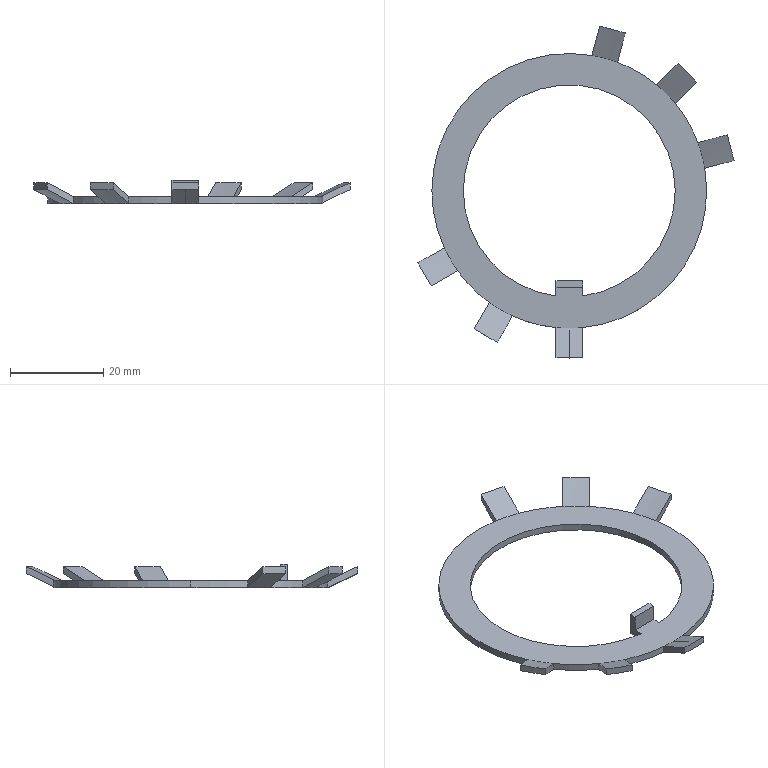Part | SolidWorks | features BaseBody 1 | 1 solid | 49 faces | box 67.906 x 71.289 x 5 mm | volume 2051 mm3 | plane 25 | cone 14 | cylinder 10 | commonest cylinder face diameters 59 x7 45.5 x3
STEP:
#1=CARTESIAN_POINT('',(0.,-29.5,0.));
#2=VERTEX_POINT('',#1);
#3=CARTESIAN_POINT('',(-2.85,-29.362,0.));
#4=VERTEX_POINT('',#3);
#5=CARTESIAN_POINT('',(0.,0.,0.));
#6=DIRECTION('',(0.,0.,-1.));
#7=DIRECTION('',(0.,1.,0.));
#8=AXIS2_PLACEMENT_3D('',#5,#6,#7);
#9=CIRCLE('',#8,29.5);
#10=EDGE_CURVE('',#2,#4,#9,.T.);
#11=ORIENTED_EDGE('',*,*,#10,.F.);
#12=CARTESIAN_POINT('',(0.,-35.887,2.978));
#13=VERTEX_POINT('',#12);
#14=CARTESIAN_POINT('',(0.,-29.5,0.));
#15=DIRECTION('',(0.,-0.9063,0.4226));
#16=VECTOR('',#15,1000.);
#17=LINE('',#14,#16);
#18=EDGE_CURVE('',#2,#13,#17,.T.);
#19=ORIENTED_EDGE('',*,*,#18,.T.);
#20=CARTESIAN_POINT('',(-2.85,-35.887,3.031));
#21=VERTEX_POINT('',#20);
#22=CARTESIAN_POINT('',(0.,-35.887,2.978));
#23=CARTESIAN_POINT('',(-0.9492,-35.887,2.978));
#24=CARTESIAN_POINT('',(-1.9,-35.887,2.996));
#25=CARTESIAN_POINT('',(-2.85,-35.887,3.031));
#26=B_SPLINE_CURVE_WITH_KNOTS('',3,(#22,#23,#24,#25),.UNSPECIFIED.,.F.,.F.,(4,4),(0.01069,0.01354),.UNSPECIFIED.);
#27=EDGE_CURVE('',#13,#21,#26,.T.);
#28=ORIENTED_EDGE('',*,*,#27,.T.);
#29=CARTESIAN_POINT('',(-2.85,-35.887,3.031));
#30=CARTESIAN_POINT('',(-2.85,-33.712,2.02));
#31=CARTESIAN_POINT('',(-2.85,-31.537,1.01));
#32=CARTESIAN_POINT('',(-2.85,-29.362,0.));
#33=B_SPLINE_CURVE_WITH_KNOTS('',3,(#29,#30,#31,#32),.UNSPECIFIED.,.F.,.F.,(4,4),(0.01329,0.02049),.UNSPECIFIED.);
#34=EDGE_CURVE('',#21,#4,#33,.T.);
#35=ORIENTED_EDGE('',*,*,#34,.T.);
#36=EDGE_LOOP('',(#11,#19,#28,#35));
#37=FACE_OUTER_BOUND('',#36,.T.);
#38=CARTESIAN_POINT('',(0.,0.,0.));
#39=DIRECTION('',(0.,0.,1.));
#40=DIRECTION('',(0.,-1.,0.));
#41=AXIS2_PLACEMENT_3D('',#38,#39,#40);
#42=CONICAL_SURFACE('',#41,29.5,1.134);
#43=ADVANCED_FACE('',(#37),#42,.T.);
#44=CARTESIAN_POINT('',(-26.853,-12.213,1.5));
#45=VERTEX_POINT('',#44);
#46=CARTESIAN_POINT('',(-29.5,0.,1.5));
#47=VERTEX_POINT('',#46);
#48=CARTESIAN_POINT('',(0.,0.,1.5));
#49=DIRECTION('',(0.,0.,-1.));
#50=DIRECTION('',(0.,1.,0.));
#51=AXIS2_PLACEMENT_3D('',#48,#49,#50);
#52=CIRCLE('',#51,29.5);
#53=EDGE_CURVE('',#45,#47,#52,.T.);
#54=ORIENTED_EDGE('',*,*,#53,.T.);
#55=CARTESIAN_POINT('',(-29.5,0.,0.));
#56=VERTEX_POINT('',#55);
#57=CARTESIAN_POINT('',(-29.5,0.,4.532));
#58=DIRECTION('',(0.,0.,-1.));
#59=VECTOR('',#58,1000.);
#60=LINE('',#57,#59);
#61=EDGE_CURVE('',#47,#56,#60,.T.);
#62=ORIENTED_EDGE('',*,*,#61,.T.);
#63=CARTESIAN_POINT('',(-26.853,-12.213,0.));
#64=VERTEX_POINT('',#63);
#65=CARTESIAN_POINT('',(0.,0.,0.));
#66=DIRECTION('',(0.,0.,1.));
#67=DIRECTION('',(1.,0.,0.));
#68=AXIS2_PLACEMENT_3D('',#65,#66,#67);
#69=CIRCLE('',#68,29.5);
#70=EDGE_CURVE('',#56,#64,#69,.T.);
#71=ORIENTED_EDGE('',*,*,#70,.T.);
#72=CARTESIAN_POINT('',(-26.853,-12.213,4.532));
#73=DIRECTION('',(0.,0.,-1.));
#74=VECTOR('',#73,1000.);
#75=LINE('',#72,#74);
#76=EDGE_CURVE('',#45,#64,#75,.T.);
#77=ORIENTED_EDGE('',*,*,#76,.F.);
#78=EDGE_LOOP('',(#54,#62,#71,#77));
#79=FACE_OUTER_BOUND('',#78,.T.);
#80=CARTESIAN_POINT('',(0.,0.,4.532));
#81=DIRECTION('',(0.,0.,-1.));
#82=DIRECTION('',(-1.,0.,0.));
#83=AXIS2_PLACEMENT_3D('',#80,#81,#82);
#84=CYLINDRICAL_SURFACE('',#83,29.5);
#85=ADVANCED_FACE('',(#79),#84,.T.);
#86=CARTESIAN_POINT('',(2.85,-22.571,1.5));
#87=VERTEX_POINT('',#86);
#88=CARTESIAN_POINT('',(22.75,0.,1.5));
#89=VERTEX_POINT('',#88);
#90=CARTESIAN_POINT('',(0.,0.,1.5));
#91=DIRECTION('',(0.,0.,1.));
#92=DIRECTION('',(0.,-1.,0.));
#93=AXIS2_PLACEMENT_3D('',#90,#91,#92);
#94=CIRCLE('',#93,22.75);
#95=EDGE_CURVE('',#87,#89,#94,.T.);
#96=ORIENTED_EDGE('',*,*,#95,.T.);
#97=CARTESIAN_POINT('',(22.75,0.,0.));
#98=VERTEX_POINT('',#97);
#99=CARTESIAN_POINT('',(22.75,0.,4.532));
#100=DIRECTION('',(0.,0.,-1.));
#101=VECTOR('',#100,1000.);
#102=LINE('',#99,#101);
#103=EDGE_CURVE('',#89,#98,#102,.T.);
#104=ORIENTED_EDGE('',*,*,#103,.T.);
#105=CARTESIAN_POINT('',(2.85,-22.571,0.));
#106=VERTEX_POINT('',#105);
#107=CARTESIAN_POINT('',(0.,0.,0.));
#108=DIRECTION('',(0.,0.,1.));
#109=DIRECTION('',(1.,0.,0.));
#110=AXIS2_PLACEMENT_3D('',#107,#108,#109);
#111=CIRCLE('',#110,22.75);
#112=EDGE_CURVE('',#106,#98,#111,.T.);
#113=ORIENTED_EDGE('',*,*,#112,.F.);
#114=CARTESIAN_POINT('',(2.85,-22.571,4.532));
#115=DIRECTION('',(0.,0.,-1.));
#116=VECTOR('',#115,1000.);
#117=LINE('',#114,#116);
#118=EDGE_CURVE('',#87,#106,#117,.T.);
#119=ORIENTED_EDGE('',*,*,#118,.F.);
#120=EDGE_LOOP('',(#96,#104,#113,#119));
#121=FACE_OUTER_BOUND('',#120,.T.);
#122=CARTESIAN_POINT('',(0.,0.,4.532));
#123=DIRECTION('',(0.,0.,-1.));
#124=DIRECTION('',(-1.,0.,0.));
#125=AXIS2_PLACEMENT_3D('',#122,#123,#124);
#126=CYLINDRICAL_SURFACE('',#125,22.75);
#127=ADVANCED_FACE('',(#121),#126,.F.);
#128=ORIENTED_EDGE('',*,*,#103,.F.);
#129=CARTESIAN_POINT('',(-22.75,0.,1.5));
#130=VERTEX_POINT('',#129);
#131=CARTESIAN_POINT('',(0.,0.,1.5));
#132=DIRECTION('',(0.,0.,1.));
#133=DIRECTION('',(0.,-1.,0.));
#134=AXIS2_PLACEMENT_3D('',#131,#132,#133);
#135=CIRCLE('',#134,22.75);
#136=EDGE_CURVE('',#89,#130,#135,.T.);
#137=ORIENTED_EDGE('',*,*,#136,.T.);
#138=CARTESIAN_POINT('',(-22.75,0.,0.));
#139=VERTEX_POINT('',#138);
#140=CARTESIAN_POINT('',(-22.75,0.,4.532));
#141=DIRECTION('',(0.,0.,-1.));
#142=VECTOR('',#141,1000.);
#143=LINE('',#140,#142);
#144=EDGE_CURVE('',#130,#139,#143,.T.);
#145=ORIENTED_EDGE('',*,*,#144,.T.);
#146=CARTESIAN_POINT('',(0.,0.,0.));
#147=DIRECTION('',(0.,0.,1.));
#148=DIRECTION('',(1.,0.,0.));
#149=AXIS2_PLACEMENT_3D('',#146,#147,#148);
#150=CIRCLE('',#149,22.75);
#151=EDGE_CURVE('',#98,#139,#150,.T.);
#152=ORIENTED_EDGE('',*,*,#151,.F.);
#153=EDGE_LOOP('',(#128,#137,#145,#152));
#154=FACE_OUTER_BOUND('',#153,.T.);
#155=CARTESIAN_POINT('',(0.,0.,4.532));
#156=DIRECTION('',(0.,0.,-1.));
#157=DIRECTION('',(-1.,0.,0.));
#158=AXIS2_PLACEMENT_3D('',#155,#156,#157);
#159=CYLINDRICAL_SURFACE('',#158,22.75);
#160=ADVANCED_FACE('',(#154),#159,.F.);
#161=CARTESIAN_POINT('',(2.85,-29.362,1.5));
#162=VERTEX_POINT('',#161);
#163=CARTESIAN_POINT('',(0.,-29.5,1.5));
#164=VERTEX_POINT('',#163);
#165=CARTESIAN_POINT('',(0.,0.,1.5));
#166=DIRECTION('',(0.,0.,-1.));
#167=DIRECTION('',(0.,1.,0.));
#168=AXIS2_PLACEMENT_3D('',#165,#166,#167);
#169=CIRCLE('',#168,29.5);
#170=EDGE_CURVE('',#162,#164,#169,.T.);
#171=ORIENTED_EDGE('',*,*,#170,.T.);
#172=CARTESIAN_POINT('',(0.,-35.887,4.478));
#173=VERTEX_POINT('',#172);
#174=CARTESIAN_POINT('',(0.,-36.,4.531));
#175=DIRECTION('',(0.,-0.9063,0.4226));
#176=VECTOR('',#175,1000.);
#177=LINE('',#174,#176);
#178=EDGE_CURVE('',#164,#173,#177,.T.);
#179=ORIENTED_EDGE('',*,*,#178,.T.);
#180=CARTESIAN_POINT('',(2.85,-35.887,4.531));
#181=VERTEX_POINT('',#180);
#182=CARTESIAN_POINT('',(0.,-35.887,4.478));
#183=CARTESIAN_POINT('',(0.951,-35.887,4.478));
#184=CARTESIAN_POINT('',(1.901,-35.887,4.496));
#185=CARTESIAN_POINT('',(2.85,-35.887,4.531));
#186=B_SPLINE_CURVE_WITH_KNOTS('',3,(#182,#183,#184,#185),.UNSPECIFIED.,.F.,.F.,(4,4),(0.01491,0.01776),.UNSPECIFIED.);
#187=EDGE_CURVE('',#173,#181,#186,.T.);
#188=ORIENTED_EDGE('',*,*,#187,.T.);
#189=CARTESIAN_POINT('',(2.85,-35.887,4.531));
#190=CARTESIAN_POINT('',(2.85,-33.712,3.52));
#191=CARTESIAN_POINT('',(2.85,-31.537,2.51));
#192=CARTESIAN_POINT('',(2.85,-29.362,1.5));
#193=B_SPLINE_CURVE_WITH_KNOTS('',3,(#189,#190,#191,#192),.UNSPECIFIED.,.F.,.F.,(4,4),(0.01329,0.02049),.UNSPECIFIED.);
#194=EDGE_CURVE('',#181,#162,#193,.T.);
#195=ORIENTED_EDGE('',*,*,#194,.T.);
#196=EDGE_LOOP('',(#171,#179,#188,#195));
#197=FACE_OUTER_BOUND('',#196,.T.);
#198=CARTESIAN_POINT('',(0.,0.,4.531));
#199=DIRECTION('',(0.,0.,1.));
#200=DIRECTION('',(0.,-1.,0.));
#201=AXIS2_PLACEMENT_3D('',#198,#199,#200);
#202=CONICAL_SURFACE('',#201,36.,1.134);
#203=ADVANCED_FACE('',(#197),#202,.F.);
#204=CARTESIAN_POINT('',(4.847,29.099,1.5));
#205=VERTEX_POINT('',#204);
#206=CARTESIAN_POINT('',(10.352,27.624,1.5));
#207=VERTEX_POINT('',#206);
#208=CARTESIAN_POINT('',(0.,0.,1.5));
#209=DIRECTION('',(0.,0.,-1.));
#210=DIRECTION('',(0.,1.,0.));
#211=AXIS2_PLACEMENT_3D('',#208,#209,#210);
#212=CIRCLE('',#211,29.5);
#213=EDGE_CURVE('',#205,#207,#212,.T.);
#214=ORIENTED_EDGE('',*,*,#213,.F.);
#215=CARTESIAN_POINT('',(0.,0.,1.5));
#216=DIRECTION('',(0.,0.,-1.));
#217=DIRECTION('',(0.,1.,0.));
#218=AXIS2_PLACEMENT_3D('',#215,#216,#217);
#219=CIRCLE('',#218,29.5);
#220=EDGE_CURVE('',#47,#205,#219,.T.);
#221=ORIENTED_EDGE('',*,*,#220,.F.);
#222=ORIENTED_EDGE('',*,*,#53,.F.);
#223=CARTESIAN_POINT('',(-24.003,-17.149,1.5));
#224=VERTEX_POINT('',#223);
#225=CARTESIAN_POINT('',(0.,0.,1.5));
#226=DIRECTION('',(0.,0.,-1.));
#227=DIRECTION('',(0.,1.,0.));
#228=AXIS2_PLACEMENT_3D('',#225,#226,#227);
#229=CIRCLE('',#228,29.5);
#230=EDGE_CURVE('',#224,#45,#229,.T.);
#231=ORIENTED_EDGE('',*,*,#230,.F.);
#232=CARTESIAN_POINT('',(-17.149,-24.003,1.5));
#233=VERTEX_POINT('',#232);
#234=CARTESIAN_POINT('',(0.,0.,1.5));
#235=DIRECTION('',(0.,0.,-1.));
#236=DIRECTION('',(0.,1.,0.));
#237=AXIS2_PLACEMENT_3D('',#234,#235,#236);
#238=CIRCLE('',#237,29.5);
#239=EDGE_CURVE('',#233,#224,#238,.T.);
#240=ORIENTED_EDGE('',*,*,#239,.F.);
#241=CARTESIAN_POINT('',(-12.213,-26.853,1.5));
#242=VERTEX_POINT('',#241);
#243=CARTESIAN_POINT('',(0.,0.,1.5));
#244=DIRECTION('',(0.,0.,-1.));
#245=DIRECTION('',(0.,1.,0.));
#246=AXIS2_PLACEMENT_3D('',#243,#244,#245);
#247=CIRCLE('',#246,29.5);
#248=EDGE_CURVE('',#242,#233,#247,.T.);
#249=ORIENTED_EDGE('',*,*,#248,.F.);
#250=CARTESIAN_POINT('',(-2.85,-29.362,1.5));
#251=VERTEX_POINT('',#250);
#252=CARTESIAN_POINT('',(0.,0.,1.5));
#253=DIRECTION('',(0.,0.,-1.));
#254=DIRECTION('',(0.,1.,0.));
#255=AXIS2_PLACEMENT_3D('',#252,#253,#254);
#256=CIRCLE('',#255,29.5);
#257=EDGE_CURVE('',#251,#242,#256,.T.);
#258=ORIENTED_EDGE('',*,*,#257,.F.);
#259=CARTESIAN_POINT('',(0.,0.,1.5));
#260=DIRECTION('',(0.,0.,-1.));
#261=DIRECTION('',(0.,1.,0.));
#262=AXIS2_PLACEMENT_3D('',#259,#260,#261);
#263=CIRCLE('',#262,29.5);
#264=EDGE_CURVE('',#164,#251,#263,.T.);
#265=ORIENTED_EDGE('',*,*,#264,.F.);
#266=ORIENTED_EDGE('',*,*,#170,.F.);
#267=CARTESIAN_POINT('',(29.099,4.847,1.5));
#268=VERTEX_POINT('',#267);
#269=CARTESIAN_POINT('',(0.,0.,1.5));
#270=DIRECTION('',(0.,0.,-1.));
#271=DIRECTION('',(0.,1.,0.));
#272=AXIS2_PLACEMENT_3D('',#269,#270,#271);
#273=CIRCLE('',#272,29.5);
#274=EDGE_CURVE('',#268,#162,#273,.T.);
#275=ORIENTED_EDGE('',*,*,#274,.F.);
#276=CARTESIAN_POINT('',(27.624,10.352,1.5));
#277=VERTEX_POINT('',#276);
#278=CARTESIAN_POINT('',(0.,0.,1.5));
#279=DIRECTION('',(0.,0.,-1.));
#280=DIRECTION('',(0.,1.,0.));
#281=AXIS2_PLACEMENT_3D('',#278,#279,#280);
#282=CIRCLE('',#281,29.5);
#283=EDGE_CURVE('',#277,#268,#282,.T.);
#284=ORIENTED_EDGE('',*,*,#283,.F.);
#285=CARTESIAN_POINT('',(22.777,18.747,1.5));
#286=VERTEX_POINT('',#285);
#287=CARTESIAN_POINT('',(0.,0.,1.5));
#288=DIRECTION('',(0.,0.,-1.));
#289=DIRECTION('',(0.,1.,0.));
#290=AXIS2_PLACEMENT_3D('',#287,#288,#289);
#291=CIRCLE('',#290,29.5);
#292=EDGE_CURVE('',#286,#277,#291,.T.);
#293=ORIENTED_EDGE('',*,*,#292,.F.);
#294=CARTESIAN_POINT('',(18.747,22.777,1.5));
#295=VERTEX_POINT('',#294);
#296=CARTESIAN_POINT('',(0.,0.,1.5));
#297=DIRECTION('',(0.,0.,-1.));
#298=DIRECTION('',(0.,1.,0.));
#299=AXIS2_PLACEMENT_3D('',#296,#297,#298);
#300=CIRCLE('',#299,29.5);
#301=EDGE_CURVE('',#295,#286,#300,.T.);
#302=ORIENTED_EDGE('',*,*,#301,.F.);
#303=CARTESIAN_POINT('',(0.,0.,1.5));
#304=DIRECTION('',(0.,0.,-1.));
#305=DIRECTION('',(0.,1.,0.));
#306=AXIS2_PLACEMENT_3D('',#303,#304,#305);
#307=CIRCLE('',#306,29.5);
#308=EDGE_CURVE('',#207,#295,#307,.T.);
#309=ORIENTED_EDGE('',*,*,#308,.F.);
#310=EDGE_LOOP('',(#214,#221,#222,#231,#240,#249,#258,#265,#266,#275,#284,#293,#302,#309));
#311=FACE_OUTER_BOUND('',#310,.T.);
#312=CARTESIAN_POINT('',(2.85,-20.75,1.5));
#313=VERTEX_POINT('',#312);
#314=CARTESIAN_POINT('',(2.85,-22.571,1.5));
#315=DIRECTION('',(0.,-1.,0.));
#316=VECTOR('',#315,1000.);
#317=LINE('',#314,#316);
#318=EDGE_CURVE('',#313,#87,#317,.T.);
#319=ORIENTED_EDGE('',*,*,#318,.F.);
#320=CARTESIAN_POINT('',(-2.85,-20.75,1.5));
#321=VERTEX_POINT('',#320);
#322=CARTESIAN_POINT('',(0.,-20.75,1.5));
#323=DIRECTION('',(-1.,0.,0.));
#324=VECTOR('',#323,1000.);
#325=LINE('',#322,#324);
#326=EDGE_CURVE('',#313,#321,#325,.T.);
#327=ORIENTED_EDGE('',*,*,#326,.T.);
#328=CARTESIAN_POINT('',(-2.85,-22.571,1.5));
#329=VERTEX_POINT('',#328);
#330=CARTESIAN_POINT('',(-2.85,-22.571,1.5));
#331=DIRECTION('',(0.,1.,0.));
#332=VECTOR('',#331,1000.);
#333=LINE('',#330,#332);
#334=EDGE_CURVE('',#329,#321,#333,.T.);
#335=ORIENTED_EDGE('',*,*,#334,.F.);
#336=CARTESIAN_POINT('',(0.,0.,1.5));
#337=DIRECTION('',(0.,0.,1.));
#338=DIRECTION('',(0.,-1.,0.));
#339=AXIS2_PLACEMENT_3D('',#336,#337,#338);
#340=CIRCLE('',#339,22.75);
#341=EDGE_CURVE('',#130,#329,#340,.T.);
#342=ORIENTED_EDGE('',*,*,#341,.F.);
#343=ORIENTED_EDGE('',*,*,#136,.F.);
#344=ORIENTED_EDGE('',*,*,#95,.F.);
#345=EDGE_LOOP('',(#319,#327,#335,#342,#343,#344));
#346=FACE_BOUND('',#345,.T.);
#347=CARTESIAN_POINT('',(0.,29.5,1.5));
#348=DIRECTION('',(0.,0.,1.));
#349=DIRECTION('',(0.,-1.,0.));
#350=AXIS2_PLACEMENT_3D('',#347,#348,#349);
#351=PLANE('',#350);
#352=ADVANCED_FACE('',(#311,#346),#351,.T.);
#353=ORIENTED_EDGE('',*,*,#178,.F.);
#354=ORIENTED_EDGE('',*,*,#264,.T.);
#355=CARTESIAN_POINT('',(-2.85,-35.887,4.531));
#356=VERTEX_POINT('',#355);
#357=CARTESIAN_POINT('',(-2.85,-29.362,1.5));
#358=CARTESIAN_POINT('',(-2.85,-31.537,2.51));
#359=CARTESIAN_POINT('',(-2.85,-33.712,3.52));
#360=CARTESIAN_POINT('',(-2.85,-35.887,4.531));
#361=B_SPLINE_CURVE_WITH_KNOTS('',3,(#357,#358,#359,#360),.UNSPECIFIED.,.F.,.F.,(4,4),(0.008218,0.01541),.UNSPECIFIED.);
#362=EDGE_CURVE('',#251,#356,#361,.T.);
#363=ORIENTED_EDGE('',*,*,#362,.T.);
#364=CARTESIAN_POINT('',(-2.85,-35.887,4.531));
#365=CARTESIAN_POINT('',(-1.9,-35.887,4.496));
#366=CARTESIAN_POINT('',(-0.9492,-35.887,4.478));
#367=CARTESIAN_POINT('',(0.,-35.887,4.478));
#368=B_SPLINE_CURVE_WITH_KNOTS('',3,(#364,#365,#366,#367),.UNSPECIFIED.,.F.,.F.,(4,4),(0.01207,0.01491),.UNSPECIFIED.);
#369=EDGE_CURVE('',#356,#173,#368,.T.);
#370=ORIENTED_EDGE('',*,*,#369,.T.);
#371=EDGE_LOOP('',(#353,#354,#363,#370));
#372=FACE_OUTER_BOUND('',#371,.T.);
#373=CARTESIAN_POINT('',(0.,0.,4.531));
#374=DIRECTION('',(0.,0.,1.));
#375=DIRECTION('',(0.,-1.,0.));
#376=AXIS2_PLACEMENT_3D('',#373,#374,#375);
#377=CONICAL_SURFACE('',#376,36.,1.134);
#378=ADVANCED_FACE('',(#372),#377,.F.);
#379=CARTESIAN_POINT('',(-20.412,-29.654,4.531));
#380=VERTEX_POINT('',#379);
#381=CARTESIAN_POINT('',(-17.149,-24.003,1.5));
#382=CARTESIAN_POINT('',(-18.237,-25.887,2.51));
#383=CARTESIAN_POINT('',(-19.324,-27.771,3.52));
#384=CARTESIAN_POINT('',(-20.412,-29.654,4.531));
#385=B_SPLINE_CURVE_WITH_KNOTS('',3,(#381,#382,#383,#384),.UNSPECIFIED.,.F.,.F.,(4,4),(0.000000255,0.007195),.UNSPECIFIED.);
#386=EDGE_CURVE('',#233,#380,#385,.T.);
#387=ORIENTED_EDGE('',*,*,#386,.T.);
#388=CARTESIAN_POINT('',(-15.475,-32.504,4.531));
#389=VERTEX_POINT('',#388);
#390=CARTESIAN_POINT('',(-20.412,-29.654,4.531));
#391=CARTESIAN_POINT('',(-18.766,-30.604,4.461));
#392=CARTESIAN_POINT('',(-17.121,-31.554,4.461));
#393=CARTESIAN_POINT('',(-15.475,-32.504,4.531));
#394=B_SPLINE_CURVE_WITH_KNOTS('',3,(#390,#391,#392,#393),.UNSPECIFIED.,.F.,.F.,(4,4),(0.000000231,0.0057),.UNSPECIFIED.);
#395=EDGE_CURVE('',#380,#389,#394,.T.);
#396=ORIENTED_EDGE('',*,*,#395,.T.);
#397=CARTESIAN_POINT('',(-15.475,-32.504,4.531));
#398=CARTESIAN_POINT('',(-14.388,-30.621,3.52));
#399=CARTESIAN_POINT('',(-13.3,-28.737,2.51));
#400=CARTESIAN_POINT('',(-12.213,-26.853,1.5));
#401=B_SPLINE_CURVE_WITH_KNOTS('',3,(#397,#398,#399,#400),.UNSPECIFIED.,.F.,.F.,(4,4),(0.000000255,0.007195),.UNSPECIFIED.);
#402=EDGE_CURVE('',#389,#242,#401,.T.);
#403=ORIENTED_EDGE('',*,*,#402,.T.);
#404=ORIENTED_EDGE('',*,*,#248,.T.);
#405=EDGE_LOOP('',(#387,#396,#403,#404));
#406=FACE_OUTER_BOUND('',#405,.T.);
#407=CARTESIAN_POINT('',(0.,0.,4.531));
#408=DIRECTION('',(0.,0.,1.));
#409=DIRECTION('',(0.,-1.,0.));
#410=AXIS2_PLACEMENT_3D('',#407,#408,#409);
#411=CONICAL_SURFACE('',#410,36.,1.134);
#412=ADVANCED_FACE('',(#406),#411,.F.);
#413=CARTESIAN_POINT('',(-32.504,-15.475,4.531));
#414=VERTEX_POINT('',#413);
#415=CARTESIAN_POINT('',(-26.853,-12.213,1.5));
#416=CARTESIAN_POINT('',(-28.737,-13.3,2.51));
#417=CARTESIAN_POINT('',(-30.621,-14.388,3.52));
#418=CARTESIAN_POINT('',(-32.504,-15.475,4.531));
#419=B_SPLINE_CURVE_WITH_KNOTS('',3,(#415,#416,#417,#418),.UNSPECIFIED.,.F.,.F.,(4,4),(0.000000255,0.007195),.UNSPECIFIED.);
#420=EDGE_CURVE('',#45,#414,#419,.T.);
#421=ORIENTED_EDGE('',*,*,#420,.T.);
#422=CARTESIAN_POINT('',(-29.654,-20.412,4.531));
#423=VERTEX_POINT('',#422);
#424=CARTESIAN_POINT('',(-32.504,-15.475,4.531));
#425=CARTESIAN_POINT('',(-31.554,-17.121,4.461));
#426=CARTESIAN_POINT('',(-30.604,-18.766,4.461));
#427=CARTESIAN_POINT('',(-29.654,-20.412,4.531));
#428=B_SPLINE_CURVE_WITH_KNOTS('',3,(#424,#425,#426,#427),.UNSPECIFIED.,.F.,.F.,(4,4),(0.000000231,0.0057),.UNSPECIFIED.);
#429=EDGE_CURVE('',#414,#423,#428,.T.);
#430=ORIENTED_EDGE('',*,*,#429,.T.);
#431=CARTESIAN_POINT('',(-29.654,-20.412,4.531));
#432=CARTESIAN_POINT('',(-27.771,-19.324,3.52));
#433=CARTESIAN_POINT('',(-25.887,-18.237,2.51));
#434=CARTESIAN_POINT('',(-24.003,-17.149,1.5));
#435=B_SPLINE_CURVE_WITH_KNOTS('',3,(#431,#432,#433,#434),.UNSPECIFIED.,.F.,.F.,(4,4),(0.000000255,0.007195),.UNSPECIFIED.);
#436=EDGE_CURVE('',#423,#224,#435,.T.);
#437=ORIENTED_EDGE('',*,*,#436,.T.);
#438=ORIENTED_EDGE('',*,*,#230,.T.);
#439=EDGE_LOOP('',(#421,#430,#437,#438));
#440=FACE_OUTER_BOUND('',#439,.T.);
#441=CARTESIAN_POINT('',(0.,0.,4.531));
#442=DIRECTION('',(0.,0.,1.));
#443=DIRECTION('',(0.,-1.,0.));
#444=AXIS2_PLACEMENT_3D('',#441,#442,#443);
#445=CONICAL_SURFACE('',#444,36.,1.134);
#446=ADVANCED_FACE('',(#440),#445,.F.);
#447=CARTESIAN_POINT('',(12.041,33.927,4.531));
#448=VERTEX_POINT('',#447);
#449=CARTESIAN_POINT('',(10.352,27.624,1.5));
#450=CARTESIAN_POINT('',(10.915,29.725,2.51));
#451=CARTESIAN_POINT('',(11.478,31.826,3.52));
#452=CARTESIAN_POINT('',(12.041,33.927,4.531));
#453=B_SPLINE_CURVE_WITH_KNOTS('',3,(#449,#450,#451,#452),.UNSPECIFIED.,.F.,.F.,(4,4),(0.000000228,0.007195),.UNSPECIFIED.);
#454=EDGE_CURVE('',#207,#448,#453,.T.);
#455=ORIENTED_EDGE('',*,*,#454,.T.);
#456=CARTESIAN_POINT('',(6.535,35.402,4.531));
#457=VERTEX_POINT('',#456);
#458=CARTESIAN_POINT('',(12.041,33.927,4.531));
#459=CARTESIAN_POINT('',(10.206,34.418,4.461));
#460=CARTESIAN_POINT('',(8.371,34.91,4.461));
#461=CARTESIAN_POINT('',(6.535,35.402,4.531));
#462=B_SPLINE_CURVE_WITH_KNOTS('',3,(#458,#459,#460,#461),.UNSPECIFIED.,.F.,.F.,(4,4),(0.000000207,0.0057),.UNSPECIFIED.);
#463=EDGE_CURVE('',#448,#457,#462,.T.);
#464=ORIENTED_EDGE('',*,*,#463,.T.);
#465=CARTESIAN_POINT('',(6.535,35.402,4.531));
#466=CARTESIAN_POINT('',(5.972,33.301,3.52));
#467=CARTESIAN_POINT('',(5.41,31.2,2.51));
#468=CARTESIAN_POINT('',(4.847,29.099,1.5));
#469=B_SPLINE_CURVE_WITH_KNOTS('',3,(#465,#466,#467,#468),.UNSPECIFIED.,.F.,.F.,(4,4),(0.000000228,0.007195),.UNSPECIFIED.);
#470=EDGE_CURVE('',#457,#205,#469,.T.);
#471=ORIENTED_EDGE('',*,*,#470,.T.);
#472=ORIENTED_EDGE('',*,*,#213,.T.);
#473=EDGE_LOOP('',(#455,#464,#471,#472));
#474=FACE_OUTER_BOUND('',#473,.T.);
#475=CARTESIAN_POINT('',(0.,0.,4.531));
#476=DIRECTION('',(0.,0.,1.));
#477=DIRECTION('',(0.,-1.,0.));
#478=AXIS2_PLACEMENT_3D('',#475,#476,#477);
#479=CONICAL_SURFACE('',#478,36.,1.134);
#480=ADVANCED_FACE('',(#474),#479,.F.);
#481=CARTESIAN_POINT('',(27.391,23.361,4.531));
#482=VERTEX_POINT('',#481);
#483=CARTESIAN_POINT('',(22.777,18.747,1.5));
#484=CARTESIAN_POINT('',(24.316,20.285,2.51));
#485=CARTESIAN_POINT('',(25.853,21.823,3.52));
#486=CARTESIAN_POINT('',(27.391,23.361,4.531));
#487=B_SPLINE_CURVE_WITH_KNOTS('',3,(#483,#484,#485,#486),.UNSPECIFIED.,.F.,.F.,(4,4),(0.000000312,0.007195),.UNSPECIFIED.);
#488=EDGE_CURVE('',#286,#482,#487,.T.);
#489=ORIENTED_EDGE('',*,*,#488,.T.);
#490=CARTESIAN_POINT('',(23.361,27.391,4.531));
#491=VERTEX_POINT('',#490);
#492=CARTESIAN_POINT('',(27.391,23.361,4.531));
#493=CARTESIAN_POINT('',(26.048,24.704,4.461));
#494=CARTESIAN_POINT('',(24.704,26.048,4.461));
#495=CARTESIAN_POINT('',(23.361,27.391,4.531));
#496=B_SPLINE_CURVE_WITH_KNOTS('',3,(#492,#493,#494,#495),.UNSPECIFIED.,.F.,.F.,(4,4),(0.000000283,0.0057),.UNSPECIFIED.);
#497=EDGE_CURVE('',#482,#491,#496,.T.);
#498=ORIENTED_EDGE('',*,*,#497,.T.);
#499=CARTESIAN_POINT('',(23.361,27.391,4.531));
#500=CARTESIAN_POINT('',(21.823,25.853,3.52));
#501=CARTESIAN_POINT('',(20.285,24.316,2.51));
#502=CARTESIAN_POINT('',(18.747,22.777,1.5));
#503=B_SPLINE_CURVE_WITH_KNOTS('',3,(#499,#500,#501,#502),.UNSPECIFIED.,.F.,.F.,(4,4),(0.000000312,0.007195),.UNSPECIFIED.);
#504=EDGE_CURVE('',#491,#295,#503,.T.);
#505=ORIENTED_EDGE('',*,*,#504,.T.);
#506=ORIENTED_EDGE('',*,*,#301,.T.);
#507=EDGE_LOOP('',(#489,#498,#505,#506));
#508=FACE_OUTER_BOUND('',#507,.T.);
#509=CARTESIAN_POINT('',(0.,0.,4.531));
#510=DIRECTION('',(0.,0.,1.));
#511=DIRECTION('',(0.,-1.,0.));
#512=AXIS2_PLACEMENT_3D('',#509,#510,#511);
#513=CONICAL_SURFACE('',#512,36.,1.134);
#514=ADVANCED_FACE('',(#508),#513,.F.);
#515=CARTESIAN_POINT('',(35.402,6.535,4.531));
#516=VERTEX_POINT('',#515);
#517=CARTESIAN_POINT('',(29.099,4.847,1.5));
#518=CARTESIAN_POINT('',(31.2,5.41,2.51));
#519=CARTESIAN_POINT('',(33.301,5.972,3.52));
#520=CARTESIAN_POINT('',(35.402,6.535,4.531));
#521=B_SPLINE_CURVE_WITH_KNOTS('',3,(#517,#518,#519,#520),.UNSPECIFIED.,.F.,.F.,(4,4),(0.000000228,0.007195),.UNSPECIFIED.);
#522=EDGE_CURVE('',#268,#516,#521,.T.);
#523=ORIENTED_EDGE('',*,*,#522,.T.);
#524=CARTESIAN_POINT('',(33.927,12.041,4.531));
#525=VERTEX_POINT('',#524);
#526=CARTESIAN_POINT('',(35.402,6.535,4.531));
#527=CARTESIAN_POINT('',(34.91,8.371,4.461));
#528=CARTESIAN_POINT('',(34.418,10.206,4.461));
#529=CARTESIAN_POINT('',(33.927,12.041,4.531));
#530=B_SPLINE_CURVE_WITH_KNOTS('',3,(#526,#527,#528,#529),.UNSPECIFIED.,.F.,.F.,(4,4),(0.000000207,0.0057),.UNSPECIFIED.);
#531=EDGE_CURVE('',#516,#525,#530,.T.);
#532=ORIENTED_EDGE('',*,*,#531,.T.);
#533=CARTESIAN_POINT('',(33.927,12.041,4.531));
#534=CARTESIAN_POINT('',(31.826,11.478,3.52));
#535=CARTESIAN_POINT('',(29.725,10.915,2.51));
#536=CARTESIAN_POINT('',(27.624,10.352,1.5));
#537=B_SPLINE_CURVE_WITH_KNOTS('',3,(#533,#534,#535,#536),.UNSPECIFIED.,.F.,.F.,(4,4),(0.000000228,0.007195),.UNSPECIFIED.);
#538=EDGE_CURVE('',#525,#277,#537,.T.);
#539=ORIENTED_EDGE('',*,*,#538,.T.);
#540=ORIENTED_EDGE('',*,*,#283,.T.);
#541=EDGE_LOOP('',(#523,#532,#539,#540));
#542=FACE_OUTER_BOUND('',#541,.T.);
#543=CARTESIAN_POINT('',(0.,0.,4.531));
#544=DIRECTION('',(0.,0.,1.));
#545=DIRECTION('',(0.,-1.,0.));
#546=AXIS2_PLACEMENT_3D('',#543,#544,#545);
#547=CONICAL_SURFACE('',#546,36.,1.134);
#548=ADVANCED_FACE('',(#542),#547,.F.);
#549=CARTESIAN_POINT('',(2.85,-19.25,5.));
#550=VERTEX_POINT('',#549);
#551=CARTESIAN_POINT('',(2.85,-19.25,0.));
#552=VERTEX_POINT('',#551);
#553=CARTESIAN_POINT('',(2.85,-19.25,4.532));
#554=DIRECTION('',(0.,0.,-1.));
#555=VECTOR('',#554,1000.);
#556=LINE('',#553,#555);
#557=EDGE_CURVE('',#550,#552,#556,.T.);
#558=ORIENTED_EDGE('',*,*,#557,.F.);
#559=CARTESIAN_POINT('',(2.85,-20.75,5.));
#560=VERTEX_POINT('',#559);
#561=CARTESIAN_POINT('',(2.85,-19.25,5.));
#562=DIRECTION('',(0.,1.,0.));
#563=VECTOR('',#562,1000.);
#564=LINE('',#561,#563);
#565=EDGE_CURVE('',#560,#550,#564,.T.);
#566=ORIENTED_EDGE('',*,*,#565,.F.);
#567=CARTESIAN_POINT('',(2.85,-20.75,5.));
#568=DIRECTION('',(0.,0.,-1.));
#569=VECTOR('',#568,1000.);
#570=LINE('',#567,#569);
#571=EDGE_CURVE('',#560,#313,#570,.T.);
#572=ORIENTED_EDGE('',*,*,#571,.T.);
#573=ORIENTED_EDGE('',*,*,#318,.T.);
#574=ORIENTED_EDGE('',*,*,#118,.T.);
#575=CARTESIAN_POINT('',(2.85,-22.571,0.));
#576=DIRECTION('',(0.,-1.,0.));
#577=VECTOR('',#576,1000.);
#578=LINE('',#575,#577);
#579=EDGE_CURVE('',#552,#106,#578,.T.);
#580=ORIENTED_EDGE('',*,*,#579,.F.);
#581=EDGE_LOOP('',(#558,#566,#572,#573,#574,#580));
#582=FACE_OUTER_BOUND('',#581,.T.);
#583=CARTESIAN_POINT('',(2.85,-22.571,4.532));
#584=DIRECTION('',(1.,0.,0.));
#585=DIRECTION('',(0.,0.,-1.));
#586=AXIS2_PLACEMENT_3D('',#583,#584,#585);
#587=PLANE('',#586);
#588=ADVANCED_FACE('',(#582),#587,.T.);
#589=CARTESIAN_POINT('',(-2.85,-19.25,5.));
#590=VERTEX_POINT('',#589);
#591=CARTESIAN_POINT('',(-2.85,-19.25,0.));
#592=VERTEX_POINT('',#591);
#593=CARTESIAN_POINT('',(-2.85,-19.25,4.532));
#594=DIRECTION('',(0.,0.,-1.));
#595=VECTOR('',#594,1000.);
#596=LINE('',#593,#595);
#597=EDGE_CURVE('',#590,#592,#596,.T.);
#598=ORIENTED_EDGE('',*,*,#597,.F.);
#599=CARTESIAN_POINT('',(-2.85,-19.25,5.));
#600=DIRECTION('',(-1.,0.,0.));
#601=VECTOR('',#600,1000.);
#602=LINE('',#599,#601);
#603=EDGE_CURVE('',#550,#590,#602,.T.);
#604=ORIENTED_EDGE('',*,*,#603,.F.);
#605=ORIENTED_EDGE('',*,*,#557,.T.);
#606=CARTESIAN_POINT('',(2.85,-19.25,0.));
#607=DIRECTION('',(1.,0.,0.));
#608=VECTOR('',#607,1000.);
#609=LINE('',#606,#608);
#610=EDGE_CURVE('',#592,#552,#609,.T.);
#611=ORIENTED_EDGE('',*,*,#610,.F.);
#612=EDGE_LOOP('',(#598,#604,#605,#611));
#613=FACE_OUTER_BOUND('',#612,.T.);
#614=CARTESIAN_POINT('',(2.85,-19.25,4.532));
#615=DIRECTION('',(0.,1.,0.));
#616=DIRECTION('',(0.,0.,1.));
#617=AXIS2_PLACEMENT_3D('',#614,#615,#616);
#618=PLANE('',#617);
#619=ADVANCED_FACE('',(#613),#618,.T.);
#620=ORIENTED_EDGE('',*,*,#597,.T.);
#621=CARTESIAN_POINT('',(-2.85,-22.571,0.));
#622=VERTEX_POINT('',#621);
#623=CARTESIAN_POINT('',(-2.85,-22.571,0.));
#624=DIRECTION('',(0.,1.,0.));
#625=VECTOR('',#624,1000.);
#626=LINE('',#623,#625);
#627=EDGE_CURVE('',#622,#592,#626,.T.);
#628=ORIENTED_EDGE('',*,*,#627,.F.);
#629=CARTESIAN_POINT('',(-2.85,-22.571,4.532));
#630=DIRECTION('',(0.,0.,-1.));
#631=VECTOR('',#630,1000.);
#632=LINE('',#629,#631);
#633=EDGE_CURVE('',#329,#622,#632,.T.);
#634=ORIENTED_EDGE('',*,*,#633,.F.);
#635=ORIENTED_EDGE('',*,*,#334,.T.);
#636=CARTESIAN_POINT('',(-2.85,-20.75,5.));
#637=VERTEX_POINT('',#636);
#638=CARTESIAN_POINT('',(-2.85,-20.75,5.));
#639=DIRECTION('',(0.,0.,-1.));
#640=VECTOR('',#639,1000.);
#641=LINE('',#638,#640);
#642=EDGE_CURVE('',#637,#321,#641,.T.);
#643=ORIENTED_EDGE('',*,*,#642,.F.);
#644=CARTESIAN_POINT('',(-2.85,-19.25,5.));
#645=DIRECTION('',(0.,-1.,0.));
#646=VECTOR('',#645,1000.);
#647=LINE('',#644,#646);
#648=EDGE_CURVE('',#590,#637,#647,.T.);
#649=ORIENTED_EDGE('',*,*,#648,.F.);
#650=EDGE_LOOP('',(#620,#628,#634,#635,#643,#649));
#651=FACE_OUTER_BOUND('',#650,.T.);
#652=CARTESIAN_POINT('',(-2.85,-22.571,4.532));
#653=DIRECTION('',(-1.,0.,0.));
#654=DIRECTION('',(0.,-1.,0.));
#655=AXIS2_PLACEMENT_3D('',#652,#653,#654);
#656=PLANE('',#655);
#657=ADVANCED_FACE('',(#651),#656,.T.);
#658=ORIENTED_EDGE('',*,*,#144,.F.);
#659=ORIENTED_EDGE('',*,*,#341,.T.);
#660=ORIENTED_EDGE('',*,*,#633,.T.);
#661=CARTESIAN_POINT('',(0.,0.,0.));
#662=DIRECTION('',(0.,0.,1.));
#663=DIRECTION('',(1.,0.,0.));
#664=AXIS2_PLACEMENT_3D('',#661,#662,#663);
#665=CIRCLE('',#664,22.75);
#666=EDGE_CURVE('',#139,#622,#665,.T.);
#667=ORIENTED_EDGE('',*,*,#666,.F.);
#668=EDGE_LOOP('',(#658,#659,#660,#667));
#669=FACE_OUTER_BOUND('',#668,.T.);
#670=CARTESIAN_POINT('',(0.,0.,4.532));
#671=DIRECTION('',(0.,0.,-1.));
#672=DIRECTION('',(-1.,0.,0.));
#673=AXIS2_PLACEMENT_3D('',#670,#671,#672);
#674=CYLINDRICAL_SURFACE('',#673,22.75);
#675=ADVANCED_FACE('',(#669),#674,.F.);
#676=CARTESIAN_POINT('',(2.85,-29.362,0.));
#677=VERTEX_POINT('',#676);
#678=CARTESIAN_POINT('',(2.85,-35.887,3.031));
#679=VERTEX_POINT('',#678);
#680=CARTESIAN_POINT('',(2.85,-29.362,0.));
#681=CARTESIAN_POINT('',(2.85,-31.537,1.01));
#682=CARTESIAN_POINT('',(2.85,-33.712,2.02));
#683=CARTESIAN_POINT('',(2.85,-35.887,3.031));
#684=B_SPLINE_CURVE_WITH_KNOTS('',3,(#680,#681,#682,#683),.UNSPECIFIED.,.F.,.F.,(4,4),(0.008218,0.01541),.UNSPECIFIED.);
#685=EDGE_CURVE('',#677,#679,#684,.T.);
#686=ORIENTED_EDGE('',*,*,#685,.F.);
#687=CARTESIAN_POINT('',(2.85,-29.362,4.532));
#688=DIRECTION('',(0.,0.,-1.));
#689=VECTOR('',#688,1000.);
#690=LINE('',#687,#689);
#691=EDGE_CURVE('',#162,#677,#690,.T.);
#692=ORIENTED_EDGE('',*,*,#691,.F.);
#693=ORIENTED_EDGE('',*,*,#194,.F.);
#694=CARTESIAN_POINT('',(2.85,-35.887,4.532));
#695=DIRECTION('',(0.,0.,-1.));
#696=VECTOR('',#695,1000.);
#697=LINE('',#694,#696);
#698=EDGE_CURVE('',#181,#679,#697,.T.);
#699=ORIENTED_EDGE('',*,*,#698,.T.);
#700=EDGE_LOOP('',(#686,#692,#693,#699));
#701=FACE_OUTER_BOUND('',#700,.T.);
#702=CARTESIAN_POINT('',(2.85,-29.362,4.532));
#703=DIRECTION('',(-1.,0.,0.));
#704=DIRECTION('',(0.,-1.,0.));
#705=AXIS2_PLACEMENT_3D('',#702,#703,#704);
#706=PLANE('',#705);
#707=ADVANCED_FACE('',(#701),#706,.F.);
#708=ORIENTED_EDGE('',*,*,#274,.T.);
#709=ORIENTED_EDGE('',*,*,#691,.T.);
#710=CARTESIAN_POINT('',(29.099,4.847,0.));
#711=VERTEX_POINT('',#710);
#712=CARTESIAN_POINT('',(0.,0.,0.));
#713=DIRECTION('',(0.,0.,1.));
#714=DIRECTION('',(1.,0.,0.));
#715=AXIS2_PLACEMENT_3D('',#712,#713,#714);
#716=CIRCLE('',#715,29.5);
#717=EDGE_CURVE('',#677,#711,#716,.T.);
#718=ORIENTED_EDGE('',*,*,#717,.T.);
#719=CARTESIAN_POINT('',(29.099,4.847,4.532));
#720=DIRECTION('',(0.,0.,-1.));
#721=VECTOR('',#720,1000.);
#722=LINE('',#719,#721);
#723=EDGE_CURVE('',#268,#711,#722,.T.);
#724=ORIENTED_EDGE('',*,*,#723,.F.);
#725=EDGE_LOOP('',(#708,#709,#718,#724));
#726=FACE_OUTER_BOUND('',#725,.T.);
#727=CARTESIAN_POINT('',(0.,0.,4.532));
#728=DIRECTION('',(0.,0.,-1.));
#729=DIRECTION('',(-1.,0.,0.));
#730=AXIS2_PLACEMENT_3D('',#727,#728,#729);
#731=CYLINDRICAL_SURFACE('',#730,29.5);
#732=ADVANCED_FACE('',(#726),#731,.T.);
#733=CARTESIAN_POINT('',(35.402,6.535,3.031));
#734=VERTEX_POINT('',#733);
#735=CARTESIAN_POINT('',(35.402,6.535,3.031));
#736=CARTESIAN_POINT('',(33.301,5.972,2.02));
#737=CARTESIAN_POINT('',(31.2,5.41,1.01));
#738=CARTESIAN_POINT('',(29.099,4.847,0.));
#739=B_SPLINE_CURVE_WITH_KNOTS('',3,(#735,#736,#737,#738),.UNSPECIFIED.,.F.,.F.,(4,4),(0.000000228,0.007195),.UNSPECIFIED.);
#740=EDGE_CURVE('',#734,#711,#739,.T.);
#741=ORIENTED_EDGE('',*,*,#740,.F.);
#742=CARTESIAN_POINT('',(35.402,6.535,4.532));
#743=DIRECTION('',(0.,0.,-1.));
#744=VECTOR('',#743,1000.);
#745=LINE('',#742,#744);
#746=EDGE_CURVE('',#516,#734,#745,.T.);
#747=ORIENTED_EDGE('',*,*,#746,.F.);
#748=ORIENTED_EDGE('',*,*,#522,.F.);
#749=ORIENTED_EDGE('',*,*,#723,.T.);
#750=EDGE_LOOP('',(#741,#747,#748,#749));
#751=FACE_OUTER_BOUND('',#750,.T.);
#752=CARTESIAN_POINT('',(29.099,4.847,4.532));
#753=DIRECTION('',(-0.2588,0.9659,0.));
#754=DIRECTION('',(-0.9659,-0.2588,0.));
#755=AXIS2_PLACEMENT_3D('',#752,#753,#754);
#756=PLANE('',#755);
#757=ADVANCED_FACE('',(#751),#756,.F.);
#758=CARTESIAN_POINT('',(33.927,12.041,3.031));
#759=VERTEX_POINT('',#758);
#760=CARTESIAN_POINT('',(33.927,12.041,3.031));
#761=CARTESIAN_POINT('',(34.418,10.206,2.961));
#762=CARTESIAN_POINT('',(34.91,8.371,2.961));
#763=CARTESIAN_POINT('',(35.402,6.535,3.031));
#764=B_SPLINE_CURVE_WITH_KNOTS('',3,(#760,#761,#762,#763),.UNSPECIFIED.,.F.,.F.,(4,4),(0.000000207,0.0057),.UNSPECIFIED.);
#765=EDGE_CURVE('',#759,#734,#764,.T.);
#766=ORIENTED_EDGE('',*,*,#765,.F.);
#767=CARTESIAN_POINT('',(33.927,12.041,4.532));
#768=DIRECTION('',(0.,0.,-1.));
#769=VECTOR('',#768,1000.);
#770=LINE('',#767,#769);
#771=EDGE_CURVE('',#525,#759,#770,.T.);
#772=ORIENTED_EDGE('',*,*,#771,.F.);
#773=ORIENTED_EDGE('',*,*,#531,.F.);
#774=ORIENTED_EDGE('',*,*,#746,.T.);
#775=EDGE_LOOP('',(#766,#772,#773,#774));
#776=FACE_OUTER_BOUND('',#775,.T.);
#777=CARTESIAN_POINT('',(33.927,12.041,4.532));
#778=DIRECTION('',(-0.9659,-0.2588,0.));
#779=DIRECTION('',(0.2588,-0.9659,0.));
#780=AXIS2_PLACEMENT_3D('',#777,#778,#779);
#781=PLANE('',#780);
#782=ADVANCED_FACE('',(#776),#781,.F.);
#783=CARTESIAN_POINT('',(27.624,10.352,0.));
#784=VERTEX_POINT('',#783);
#785=CARTESIAN_POINT('',(27.624,10.352,0.));
#786=CARTESIAN_POINT('',(29.725,10.915,1.01));
#787=CARTESIAN_POINT('',(31.826,11.478,2.02));
#788=CARTESIAN_POINT('',(33.927,12.041,3.031));
#789=B_SPLINE_CURVE_WITH_KNOTS('',3,(#785,#786,#787,#788),.UNSPECIFIED.,.F.,.F.,(4,4),(0.000000228,0.007195),.UNSPECIFIED.);
#790=EDGE_CURVE('',#784,#759,#789,.T.);
#791=ORIENTED_EDGE('',*,*,#790,.F.);
#792=CARTESIAN_POINT('',(27.624,10.352,4.532));
#793=DIRECTION('',(0.,0.,-1.));
#794=VECTOR('',#793,1000.);
#795=LINE('',#792,#794);
#796=EDGE_CURVE('',#277,#784,#795,.T.);
#797=ORIENTED_EDGE('',*,*,#796,.F.);
#798=ORIENTED_EDGE('',*,*,#538,.F.);
#799=ORIENTED_EDGE('',*,*,#771,.T.);
#800=EDGE_LOOP('',(#791,#797,#798,#799));
#801=FACE_OUTER_BOUND('',#800,.T.);
#802=CARTESIAN_POINT('',(27.624,10.352,4.532));
#803=DIRECTION('',(0.2588,-0.9659,0.));
#804=DIRECTION('',(0.9659,0.2588,0.));
#805=AXIS2_PLACEMENT_3D('',#802,#803,#804);
#806=PLANE('',#805);
#807=ADVANCED_FACE('',(#801),#806,.F.);
#808=ORIENTED_EDGE('',*,*,#292,.T.);
#809=ORIENTED_EDGE('',*,*,#796,.T.);
#810=CARTESIAN_POINT('',(22.777,18.747,0.));
#811=VERTEX_POINT('',#810);
#812=CARTESIAN_POINT('',(0.,0.,0.));
#813=DIRECTION('',(0.,0.,1.));
#814=DIRECTION('',(1.,0.,0.));
#815=AXIS2_PLACEMENT_3D('',#812,#813,#814);
#816=CIRCLE('',#815,29.5);
#817=EDGE_CURVE('',#784,#811,#816,.T.);
#818=ORIENTED_EDGE('',*,*,#817,.T.);
#819=CARTESIAN_POINT('',(22.777,18.747,4.532));
#820=DIRECTION('',(0.,0.,-1.));
#821=VECTOR('',#820,1000.);
#822=LINE('',#819,#821);
#823=EDGE_CURVE('',#286,#811,#822,.T.);
#824=ORIENTED_EDGE('',*,*,#823,.F.);
#825=EDGE_LOOP('',(#808,#809,#818,#824));
#826=FACE_OUTER_BOUND('',#825,.T.);
#827=CARTESIAN_POINT('',(0.,0.,4.532));
#828=DIRECTION('',(0.,0.,-1.));
#829=DIRECTION('',(-1.,0.,0.));
#830=AXIS2_PLACEMENT_3D('',#827,#828,#829);
#831=CYLINDRICAL_SURFACE('',#830,29.5);
#832=ADVANCED_FACE('',(#826),#831,.T.);
#833=CARTESIAN_POINT('',(27.391,23.361,3.031));
#834=VERTEX_POINT('',#833);
#835=CARTESIAN_POINT('',(27.391,23.361,3.031));
#836=CARTESIAN_POINT('',(25.853,21.823,2.02));
#837=CARTESIAN_POINT('',(24.316,20.285,1.01));
#838=CARTESIAN_POINT('',(22.777,18.747,0.));
#839=B_SPLINE_CURVE_WITH_KNOTS('',3,(#835,#836,#837,#838),.UNSPECIFIED.,.F.,.F.,(4,4),(0.000000312,0.007195),.UNSPECIFIED.);
#840=EDGE_CURVE('',#834,#811,#839,.T.);
#841=ORIENTED_EDGE('',*,*,#840,.F.);
#842=CARTESIAN_POINT('',(27.391,23.361,4.532));
#843=DIRECTION('',(0.,0.,-1.));
#844=VECTOR('',#843,1000.);
#845=LINE('',#842,#844);
#846=EDGE_CURVE('',#482,#834,#845,.T.);
#847=ORIENTED_EDGE('',*,*,#846,.F.);
#848=ORIENTED_EDGE('',*,*,#488,.F.);
#849=ORIENTED_EDGE('',*,*,#823,.T.);
#850=EDGE_LOOP('',(#841,#847,#848,#849));
#851=FACE_OUTER_BOUND('',#850,.T.);
#852=CARTESIAN_POINT('',(22.777,18.747,4.532));
#853=DIRECTION('',(-0.7071,0.7071,0.));
#854=DIRECTION('',(-0.7071,-0.7071,0.));
#855=AXIS2_PLACEMENT_3D('',#852,#853,#854);
#856=PLANE('',#855);
#857=ADVANCED_FACE('',(#851),#856,.F.);
#858=CARTESIAN_POINT('',(23.361,27.391,3.031));
#859=VERTEX_POINT('',#858);
#860=CARTESIAN_POINT('',(23.361,27.391,3.031));
#861=CARTESIAN_POINT('',(24.704,26.048,2.961));
#862=CARTESIAN_POINT('',(26.048,24.704,2.961));
#863=CARTESIAN_POINT('',(27.391,23.361,3.031));
#864=B_SPLINE_CURVE_WITH_KNOTS('',3,(#860,#861,#862,#863),.UNSPECIFIED.,.F.,.F.,(4,4),(0.000000283,0.0057),.UNSPECIFIED.);
#865=EDGE_CURVE('',#859,#834,#864,.T.);
#866=ORIENTED_EDGE('',*,*,#865,.F.);
#867=CARTESIAN_POINT('',(23.361,27.391,4.532));
#868=DIRECTION('',(0.,0.,-1.));
#869=VECTOR('',#868,1000.);
#870=LINE('',#867,#869);
#871=EDGE_CURVE('',#491,#859,#870,.T.);
#872=ORIENTED_EDGE('',*,*,#871,.F.);
#873=ORIENTED_EDGE('',*,*,#497,.F.);
#874=ORIENTED_EDGE('',*,*,#846,.T.);
#875=EDGE_LOOP('',(#866,#872,#873,#874));
#876=FACE_OUTER_BOUND('',#875,.T.);
#877=CARTESIAN_POINT('',(23.361,27.391,4.532));
#878=DIRECTION('',(-0.7071,-0.7071,0.));
#879=DIRECTION('',(0.7071,-0.7071,0.));
#880=AXIS2_PLACEMENT_3D('',#877,#878,#879);
#881=PLANE('',#880);
#882=ADVANCED_FACE('',(#876),#881,.F.);
#883=CARTESIAN_POINT('',(18.747,22.777,0.));
#884=VERTEX_POINT('',#883);
#885=CARTESIAN_POINT('',(18.747,22.777,0.));
#886=CARTESIAN_POINT('',(20.285,24.316,1.01));
#887=CARTESIAN_POINT('',(21.823,25.853,2.02));
#888=CARTESIAN_POINT('',(23.361,27.391,3.031));
#889=B_SPLINE_CURVE_WITH_KNOTS('',3,(#885,#886,#887,#888),.UNSPECIFIED.,.F.,.F.,(4,4),(0.000000312,0.007195),.UNSPECIFIED.);
#890=EDGE_CURVE('',#884,#859,#889,.T.);
#891=ORIENTED_EDGE('',*,*,#890,.F.);
#892=CARTESIAN_POINT('',(18.747,22.777,4.532));
#893=DIRECTION('',(0.,0.,-1.));
#894=VECTOR('',#893,1000.);
#895=LINE('',#892,#894);
#896=EDGE_CURVE('',#295,#884,#895,.T.);
#897=ORIENTED_EDGE('',*,*,#896,.F.);
#898=ORIENTED_EDGE('',*,*,#504,.F.);
#899=ORIENTED_EDGE('',*,*,#871,.T.);
#900=EDGE_LOOP('',(#891,#897,#898,#899));
#901=FACE_OUTER_BOUND('',#900,.T.);
#902=CARTESIAN_POINT('',(18.747,22.777,4.532));
#903=DIRECTION('',(0.7071,-0.7071,0.));
#904=DIRECTION('',(0.7071,0.7071,0.));
#905=AXIS2_PLACEMENT_3D('',#902,#903,#904);
#906=PLANE('',#905);
#907=ADVANCED_FACE('',(#901),#906,.F.);
#908=ORIENTED_EDGE('',*,*,#308,.T.);
#909=ORIENTED_EDGE('',*,*,#896,.T.);
#910=CARTESIAN_POINT('',(10.352,27.624,0.));
#911=VERTEX_POINT('',#910);
#912=CARTESIAN_POINT('',(0.,0.,0.));
#913=DIRECTION('',(0.,0.,1.));
#914=DIRECTION('',(1.,0.,0.));
#915=AXIS2_PLACEMENT_3D('',#912,#913,#914);
#916=CIRCLE('',#915,29.5);
#917=EDGE_CURVE('',#884,#911,#916,.T.);
#918=ORIENTED_EDGE('',*,*,#917,.T.);
#919=CARTESIAN_POINT('',(10.352,27.624,4.532));
#920=DIRECTION('',(0.,0.,-1.));
#921=VECTOR('',#920,1000.);
#922=LINE('',#919,#921);
#923=EDGE_CURVE('',#207,#911,#922,.T.);
#924=ORIENTED_EDGE('',*,*,#923,.F.);
#925=EDGE_LOOP('',(#908,#909,#918,#924));
#926=FACE_OUTER_BOUND('',#925,.T.);
#927=CARTESIAN_POINT('',(0.,0.,4.532));
#928=DIRECTION('',(0.,0.,-1.));
#929=DIRECTION('',(-1.,0.,0.));
#930=AXIS2_PLACEMENT_3D('',#927,#928,#929);
#931=CYLINDRICAL_SURFACE('',#930,29.5);
#932=ADVANCED_FACE('',(#926),#931,.T.);
#933=CARTESIAN_POINT('',(12.041,33.927,3.031));
#934=VERTEX_POINT('',#933);
#935=CARTESIAN_POINT('',(12.041,33.927,3.031));
#936=CARTESIAN_POINT('',(11.478,31.826,2.02));
#937=CARTESIAN_POINT('',(10.915,29.725,1.01));
#938=CARTESIAN_POINT('',(10.352,27.624,0.));
#939=B_SPLINE_CURVE_WITH_KNOTS('',3,(#935,#936,#937,#938),.UNSPECIFIED.,.F.,.F.,(4,4),(0.000000228,0.007195),.UNSPECIFIED.);
#940=EDGE_CURVE('',#934,#911,#939,.T.);
#941=ORIENTED_EDGE('',*,*,#940,.F.);
#942=CARTESIAN_POINT('',(12.041,33.927,4.532));
#943=DIRECTION('',(0.,0.,-1.));
#944=VECTOR('',#943,1000.);
#945=LINE('',#942,#944);
#946=EDGE_CURVE('',#448,#934,#945,.T.);
#947=ORIENTED_EDGE('',*,*,#946,.F.);
#948=ORIENTED_EDGE('',*,*,#454,.F.);
#949=ORIENTED_EDGE('',*,*,#923,.T.);
#950=EDGE_LOOP('',(#941,#947,#948,#949));
#951=FACE_OUTER_BOUND('',#950,.T.);
#952=CARTESIAN_POINT('',(12.041,33.927,4.532));
#953=DIRECTION('',(-0.9659,0.2588,0.));
#954=DIRECTION('',(-0.2588,-0.9659,0.));
#955=AXIS2_PLACEMENT_3D('',#952,#953,#954);
#956=PLANE('',#955);
#957=ADVANCED_FACE('',(#951),#956,.F.);
#958=CARTESIAN_POINT('',(6.535,35.402,3.031));
#959=VERTEX_POINT('',#958);
#960=CARTESIAN_POINT('',(6.535,35.402,3.031));
#961=CARTESIAN_POINT('',(8.371,34.91,2.961));
#962=CARTESIAN_POINT('',(10.206,34.418,2.961));
#963=CARTESIAN_POINT('',(12.041,33.927,3.031));
#964=B_SPLINE_CURVE_WITH_KNOTS('',3,(#960,#961,#962,#963),.UNSPECIFIED.,.F.,.F.,(4,4),(0.000000207,0.0057),.UNSPECIFIED.);
#965=EDGE_CURVE('',#959,#934,#964,.T.);
#966=ORIENTED_EDGE('',*,*,#965,.F.);
#967=CARTESIAN_POINT('',(6.535,35.402,4.532));
#968=DIRECTION('',(0.,0.,-1.));
#969=VECTOR('',#968,1000.);
#970=LINE('',#967,#969);
#971=EDGE_CURVE('',#457,#959,#970,.T.);
#972=ORIENTED_EDGE('',*,*,#971,.F.);
#973=ORIENTED_EDGE('',*,*,#463,.F.);
#974=ORIENTED_EDGE('',*,*,#946,.T.);
#975=EDGE_LOOP('',(#966,#972,#973,#974));
#976=FACE_OUTER_BOUND('',#975,.T.);
#977=CARTESIAN_POINT('',(6.535,35.402,4.532));
#978=DIRECTION('',(-0.2588,-0.9659,0.));
#979=DIRECTION('',(0.9659,-0.2588,0.));
#980=AXIS2_PLACEMENT_3D('',#977,#978,#979);
#981=PLANE('',#980);
#982=ADVANCED_FACE('',(#976),#981,.F.);
#983=CARTESIAN_POINT('',(4.847,29.099,0.));
#984=VERTEX_POINT('',#983);
#985=CARTESIAN_POINT('',(4.847,29.099,0.));
#986=CARTESIAN_POINT('',(5.41,31.2,1.01));
#987=CARTESIAN_POINT('',(5.972,33.301,2.02));
#988=CARTESIAN_POINT('',(6.535,35.402,3.031));
#989=B_SPLINE_CURVE_WITH_KNOTS('',3,(#985,#986,#987,#988),.UNSPECIFIED.,.F.,.F.,(4,4),(0.000000228,0.007195),.UNSPECIFIED.);
#990=EDGE_CURVE('',#984,#959,#989,.T.);
#991=ORIENTED_EDGE('',*,*,#990,.F.);
#992=CARTESIAN_POINT('',(4.847,29.099,4.532));
#993=DIRECTION('',(0.,0.,-1.));
#994=VECTOR('',#993,1000.);
#995=LINE('',#992,#994);
#996=EDGE_CURVE('',#205,#984,#995,.T.);
#997=ORIENTED_EDGE('',*,*,#996,.F.);
#998=ORIENTED_EDGE('',*,*,#470,.F.);
#999=ORIENTED_EDGE('',*,*,#971,.T.);
#1000=EDGE_LOOP('',(#991,#997,#998,#999));
#1001=FACE_OUTER_BOUND('',#1000,.T.);
#1002=CARTESIAN_POINT('',(6.535,35.402,4.532));
#1003=DIRECTION('',(0.9659,-0.2588,0.));
#1004=DIRECTION('',(0.2588,0.9659,0.));
#1005=AXIS2_PLACEMENT_3D('',#1002,#1003,#1004);
#1006=PLANE('',#1005);
#1007=ADVANCED_FACE('',(#1001),#1006,.F.);
#1008=ORIENTED_EDGE('',*,*,#61,.F.);
#1009=ORIENTED_EDGE('',*,*,#220,.T.);
#1010=ORIENTED_EDGE('',*,*,#996,.T.);
#1011=CARTESIAN_POINT('',(0.,0.,0.));
#1012=DIRECTION('',(0.,0.,1.));
#1013=DIRECTION('',(1.,0.,0.));
#1014=AXIS2_PLACEMENT_3D('',#1011,#1012,#1013);
#1015=CIRCLE('',#1014,29.5);
#1016=EDGE_CURVE('',#984,#56,#1015,.T.);
#1017=ORIENTED_EDGE('',*,*,#1016,.T.);
#1018=EDGE_LOOP('',(#1008,#1009,#1010,#1017));
#1019=FACE_OUTER_BOUND('',#1018,.T.);
#1020=CARTESIAN_POINT('',(0.,0.,4.532));
#1021=DIRECTION('',(0.,0.,-1.));
#1022=DIRECTION('',(-1.,0.,0.));
#1023=AXIS2_PLACEMENT_3D('',#1020,#1021,#1022);
#1024=CYLINDRICAL_SURFACE('',#1023,29.5);
#1025=ADVANCED_FACE('',(#1019),#1024,.T.);
#1026=CARTESIAN_POINT('',(-32.504,-15.475,3.031));
#1027=VERTEX_POINT('',#1026);
#1028=CARTESIAN_POINT('',(-32.504,-15.475,3.031));
#1029=CARTESIAN_POINT('',(-30.621,-14.388,2.02));
#1030=CARTESIAN_POINT('',(-28.737,-13.3,1.01));
#1031=CARTESIAN_POINT('',(-26.853,-12.213,0.));
#1032=B_SPLINE_CURVE_WITH_KNOTS('',3,(#1028,#1029,#1030,#1031),.UNSPECIFIED.,.F.,.F.,(4,4),(0.000000255,0.007195),.UNSPECIFIED.);
#1033=EDGE_CURVE('',#1027,#64,#1032,.T.);
#1034=ORIENTED_EDGE('',*,*,#1033,.F.);
#1035=CARTESIAN_POINT('',(-32.504,-15.475,4.532));
#1036=DIRECTION('',(0.,0.,-1.));
#1037=VECTOR('',#1036,1000.);
#1038=LINE('',#1035,#1037);
#1039=EDGE_CURVE('',#414,#1027,#1038,.T.);
#1040=ORIENTED_EDGE('',*,*,#1039,.F.);
#1041=ORIENTED_EDGE('',*,*,#420,.F.);
#1042=ORIENTED_EDGE('',*,*,#76,.T.);
#1043=EDGE_LOOP('',(#1034,#1040,#1041,#1042));
#1044=FACE_OUTER_BOUND('',#1043,.T.);
#1045=CARTESIAN_POINT('',(-26.853,-12.213,4.532));
#1046=DIRECTION('',(0.5,-0.866,0.));
#1047=DIRECTION('',(0.866,0.5,0.));
#1048=AXIS2_PLACEMENT_3D('',#1045,#1046,#1047);
#1049=PLANE('',#1048);
#1050=ADVANCED_FACE('',(#1044),#1049,.F.);
#1051=CARTESIAN_POINT('',(-29.654,-20.412,3.031));
#1052=VERTEX_POINT('',#1051);
#1053=CARTESIAN_POINT('',(-29.654,-20.412,3.031));
#1054=CARTESIAN_POINT('',(-30.604,-18.766,2.961));
#1055=CARTESIAN_POINT('',(-31.554,-17.121,2.961));
#1056=CARTESIAN_POINT('',(-32.504,-15.475,3.031));
#1057=B_SPLINE_CURVE_WITH_KNOTS('',3,(#1053,#1054,#1055,#1056),.UNSPECIFIED.,.F.,.F.,(4,4),(0.000000231,0.0057),.UNSPECIFIED.);
#1058=EDGE_CURVE('',#1052,#1027,#1057,.T.);
#1059=ORIENTED_EDGE('',*,*,#1058,.F.);
#1060=CARTESIAN_POINT('',(-29.654,-20.412,4.532));
#1061=DIRECTION('',(0.,0.,-1.));
#1062=VECTOR('',#1061,1000.);
#1063=LINE('',#1060,#1062);
#1064=EDGE_CURVE('',#423,#1052,#1063,.T.);
#1065=ORIENTED_EDGE('',*,*,#1064,.F.);
#1066=ORIENTED_EDGE('',*,*,#429,.F.);
#1067=ORIENTED_EDGE('',*,*,#1039,.T.);
#1068=EDGE_LOOP('',(#1059,#1065,#1066,#1067));
#1069=FACE_OUTER_BOUND('',#1068,.T.);
#1070=CARTESIAN_POINT('',(-29.654,-20.412,4.532));
#1071=DIRECTION('',(0.866,0.5,0.));
#1072=DIRECTION('',(-0.5,0.866,0.));
#1073=AXIS2_PLACEMENT_3D('',#1070,#1071,#1072);
#1074=PLANE('',#1073);
#1075=ADVANCED_FACE('',(#1069),#1074,.F.);
#1076=CARTESIAN_POINT('',(-24.003,-17.149,0.));
#1077=VERTEX_POINT('',#1076);
#1078=CARTESIAN_POINT('',(-24.003,-17.149,0.));
#1079=CARTESIAN_POINT('',(-25.887,-18.237,1.01));
#1080=CARTESIAN_POINT('',(-27.771,-19.324,2.02));
#1081=CARTESIAN_POINT('',(-29.654,-20.412,3.031));
#1082=B_SPLINE_CURVE_WITH_KNOTS('',3,(#1078,#1079,#1080,#1081),.UNSPECIFIED.,.F.,.F.,(4,4),(0.000000255,0.007195),.UNSPECIFIED.);
#1083=EDGE_CURVE('',#1077,#1052,#1082,.T.);
#1084=ORIENTED_EDGE('',*,*,#1083,.F.);
#1085=CARTESIAN_POINT('',(-24.003,-17.149,4.532));
#1086=DIRECTION('',(0.,0.,-1.));
#1087=VECTOR('',#1086,1000.);
#1088=LINE('',#1085,#1087);
#1089=EDGE_CURVE('',#224,#1077,#1088,.T.);
#1090=ORIENTED_EDGE('',*,*,#1089,.F.);
#1091=ORIENTED_EDGE('',*,*,#436,.F.);
#1092=ORIENTED_EDGE('',*,*,#1064,.T.);
#1093=EDGE_LOOP('',(#1084,#1090,#1091,#1092));
#1094=FACE_OUTER_BOUND('',#1093,.T.);
#1095=CARTESIAN_POINT('',(-24.003,-17.149,4.532));
#1096=DIRECTION('',(-0.5,0.866,0.));
#1097=DIRECTION('',(-0.866,-0.5,0.));
#1098=AXIS2_PLACEMENT_3D('',#1095,#1096,#1097);
#1099=PLANE('',#1098);
#1100=ADVANCED_FACE('',(#1094),#1099,.F.);
#1101=ORIENTED_EDGE('',*,*,#239,.T.);
#1102=ORIENTED_EDGE('',*,*,#1089,.T.);
#1103=CARTESIAN_POINT('',(-17.149,-24.003,0.));
#1104=VERTEX_POINT('',#1103);
#1105=CARTESIAN_POINT('',(0.,0.,0.));
#1106=DIRECTION('',(0.,0.,1.));
#1107=DIRECTION('',(1.,0.,0.));
#1108=AXIS2_PLACEMENT_3D('',#1105,#1106,#1107);
#1109=CIRCLE('',#1108,29.5);
#1110=EDGE_CURVE('',#1077,#1104,#1109,.T.);
#1111=ORIENTED_EDGE('',*,*,#1110,.T.);
#1112=CARTESIAN_POINT('',(-17.149,-24.003,4.532));
#1113=DIRECTION('',(0.,0.,-1.));
#1114=VECTOR('',#1113,1000.);
#1115=LINE('',#1112,#1114);
#1116=EDGE_CURVE('',#233,#1104,#1115,.T.);
#1117=ORIENTED_EDGE('',*,*,#1116,.F.);
#1118=EDGE_LOOP('',(#1101,#1102,#1111,#1117));
#1119=FACE_OUTER_BOUND('',#1118,.T.);
#1120=CARTESIAN_POINT('',(0.,0.,4.532));
#1121=DIRECTION('',(0.,0.,-1.));
#1122=DIRECTION('',(-1.,0.,0.));
#1123=AXIS2_PLACEMENT_3D('',#1120,#1121,#1122);
#1124=CYLINDRICAL_SURFACE('',#1123,29.5);
#1125=ADVANCED_FACE('',(#1119),#1124,.T.);
#1126=CARTESIAN_POINT('',(-20.412,-29.654,3.031));
#1127=VERTEX_POINT('',#1126);
#1128=CARTESIAN_POINT('',(-20.412,-29.654,3.031));
#1129=CARTESIAN_POINT('',(-19.324,-27.771,2.02));
#1130=CARTESIAN_POINT('',(-18.237,-25.887,1.01));
#1131=CARTESIAN_POINT('',(-17.149,-24.003,0.));
#1132=B_SPLINE_CURVE_WITH_KNOTS('',3,(#1128,#1129,#1130,#1131),.UNSPECIFIED.,.F.,.F.,(4,4),(0.000000255,0.007195),.UNSPECIFIED.);
#1133=EDGE_CURVE('',#1127,#1104,#1132,.T.);
#1134=ORIENTED_EDGE('',*,*,#1133,.F.);
#1135=CARTESIAN_POINT('',(-20.412,-29.654,4.532));
#1136=DIRECTION('',(0.,0.,-1.));
#1137=VECTOR('',#1136,1000.);
#1138=LINE('',#1135,#1137);
#1139=EDGE_CURVE('',#380,#1127,#1138,.T.);
#1140=ORIENTED_EDGE('',*,*,#1139,.F.);
#1141=ORIENTED_EDGE('',*,*,#386,.F.);
#1142=ORIENTED_EDGE('',*,*,#1116,.T.);
#1143=EDGE_LOOP('',(#1134,#1140,#1141,#1142));
#1144=FACE_OUTER_BOUND('',#1143,.T.);
#1145=CARTESIAN_POINT('',(-20.412,-29.654,4.532));
#1146=DIRECTION('',(0.866,-0.5,0.));
#1147=DIRECTION('',(0.5,0.866,0.));
#1148=AXIS2_PLACEMENT_3D('',#1145,#1146,#1147);
#1149=PLANE('',#1148);
#1150=ADVANCED_FACE('',(#1144),#1149,.F.);
#1151=CARTESIAN_POINT('',(-15.475,-32.504,3.031));
#1152=VERTEX_POINT('',#1151);
#1153=CARTESIAN_POINT('',(-15.475,-32.504,3.031));
#1154=CARTESIAN_POINT('',(-17.121,-31.554,2.961));
#1155=CARTESIAN_POINT('',(-18.766,-30.604,2.961));
#1156=CARTESIAN_POINT('',(-20.412,-29.654,3.031));
#1157=B_SPLINE_CURVE_WITH_KNOTS('',3,(#1153,#1154,#1155,#1156),.UNSPECIFIED.,.F.,.F.,(4,4),(0.000000231,0.0057),.UNSPECIFIED.);
#1158=EDGE_CURVE('',#1152,#1127,#1157,.T.);
#1159=ORIENTED_EDGE('',*,*,#1158,.F.);
#1160=CARTESIAN_POINT('',(-15.475,-32.504,4.532));
#1161=DIRECTION('',(0.,0.,-1.));
#1162=VECTOR('',#1161,1000.);
#1163=LINE('',#1160,#1162);
#1164=EDGE_CURVE('',#389,#1152,#1163,.T.);
#1165=ORIENTED_EDGE('',*,*,#1164,.F.);
#1166=ORIENTED_EDGE('',*,*,#395,.F.);
#1167=ORIENTED_EDGE('',*,*,#1139,.T.);
#1168=EDGE_LOOP('',(#1159,#1165,#1166,#1167));
#1169=FACE_OUTER_BOUND('',#1168,.T.);
#1170=CARTESIAN_POINT('',(-20.412,-29.654,4.532));
#1171=DIRECTION('',(0.5,0.866,0.));
#1172=DIRECTION('',(-0.866,0.5,0.));
#1173=AXIS2_PLACEMENT_3D('',#1170,#1171,#1172);
#1174=PLANE('',#1173);
#1175=ADVANCED_FACE('',(#1169),#1174,.F.);
#1176=CARTESIAN_POINT('',(-12.213,-26.853,0.));
#1177=VERTEX_POINT('',#1176);
#1178=CARTESIAN_POINT('',(-12.213,-26.853,0.));
#1179=CARTESIAN_POINT('',(-13.3,-28.737,1.01));
#1180=CARTESIAN_POINT('',(-14.388,-30.621,2.02));
#1181=CARTESIAN_POINT('',(-15.475,-32.504,3.031));
#1182=B_SPLINE_CURVE_WITH_KNOTS('',3,(#1178,#1179,#1180,#1181),.UNSPECIFIED.,.F.,.F.,(4,4),(0.000000255,0.007195),.UNSPECIFIED.);
#1183=EDGE_CURVE('',#1177,#1152,#1182,.T.);
#1184=ORIENTED_EDGE('',*,*,#1183,.F.);
#1185=CARTESIAN_POINT('',(-12.213,-26.853,4.532));
#1186=DIRECTION('',(0.,0.,-1.));
#1187=VECTOR('',#1186,1000.);
#1188=LINE('',#1185,#1187);
#1189=EDGE_CURVE('',#242,#1177,#1188,.T.);
#1190=ORIENTED_EDGE('',*,*,#1189,.F.);
#1191=ORIENTED_EDGE('',*,*,#402,.F.);
#1192=ORIENTED_EDGE('',*,*,#1164,.T.);
#1193=EDGE_LOOP('',(#1184,#1190,#1191,#1192));
#1194=FACE_OUTER_BOUND('',#1193,.T.);
#1195=CARTESIAN_POINT('',(-15.475,-32.504,4.532));
#1196=DIRECTION('',(-0.866,0.5,0.));
#1197=DIRECTION('',(-0.5,-0.866,0.));
#1198=AXIS2_PLACEMENT_3D('',#1195,#1196,#1197);
#1199=PLANE('',#1198);
#1200=ADVANCED_FACE('',(#1194),#1199,.F.);
#1201=ORIENTED_EDGE('',*,*,#257,.T.);
#1202=ORIENTED_EDGE('',*,*,#1189,.T.);
#1203=CARTESIAN_POINT('',(0.,0.,0.));
#1204=DIRECTION('',(0.,0.,1.));
#1205=DIRECTION('',(1.,0.,0.));
#1206=AXIS2_PLACEMENT_3D('',#1203,#1204,#1205);
#1207=CIRCLE('',#1206,29.5);
#1208=EDGE_CURVE('',#1177,#4,#1207,.T.);
#1209=ORIENTED_EDGE('',*,*,#1208,.T.);
#1210=CARTESIAN_POINT('',(-2.85,-29.362,4.532));
#1211=DIRECTION('',(0.,0.,-1.));
#1212=VECTOR('',#1211,1000.);
#1213=LINE('',#1210,#1212);
#1214=EDGE_CURVE('',#251,#4,#1213,.T.);
#1215=ORIENTED_EDGE('',*,*,#1214,.F.);
#1216=EDGE_LOOP('',(#1201,#1202,#1209,#1215));
#1217=FACE_OUTER_BOUND('',#1216,.T.);
#1218=CARTESIAN_POINT('',(0.,0.,4.532));
#1219=DIRECTION('',(0.,0.,-1.));
#1220=DIRECTION('',(-1.,0.,0.));
#1221=AXIS2_PLACEMENT_3D('',#1218,#1219,#1220);
#1222=CYLINDRICAL_SURFACE('',#1221,29.5);
#1223=ADVANCED_FACE('',(#1217),#1222,.T.);
#1224=ORIENTED_EDGE('',*,*,#34,.F.);
#1225=CARTESIAN_POINT('',(-2.85,-35.887,4.532));
#1226=DIRECTION('',(0.,0.,-1.));
#1227=VECTOR('',#1226,1000.);
#1228=LINE('',#1225,#1227);
#1229=EDGE_CURVE('',#356,#21,#1228,.T.);
#1230=ORIENTED_EDGE('',*,*,#1229,.F.);
#1231=ORIENTED_EDGE('',*,*,#362,.F.);
#1232=ORIENTED_EDGE('',*,*,#1214,.T.);
#1233=EDGE_LOOP('',(#1224,#1230,#1231,#1232));
#1234=FACE_OUTER_BOUND('',#1233,.T.);
#1235=CARTESIAN_POINT('',(-2.85,-29.362,4.532));
#1236=DIRECTION('',(1.,0.,0.));
#1237=DIRECTION('',(0.,1.,0.));
#1238=AXIS2_PLACEMENT_3D('',#1235,#1236,#1237);
#1239=PLANE('',#1238);
#1240=ADVANCED_FACE('',(#1234),#1239,.F.);
#1241=CARTESIAN_POINT('',(2.85,-35.887,3.031));
#1242=CARTESIAN_POINT('',(1.901,-35.887,2.996));
#1243=CARTESIAN_POINT('',(0.951,-35.887,2.978));
#1244=CARTESIAN_POINT('',(0.,-35.887,2.978));
#1245=B_SPLINE_CURVE_WITH_KNOTS('',3,(#1241,#1242,#1243,#1244),.UNSPECIFIED.,.F.,.F.,(4,4),(0.007845,0.01069),.UNSPECIFIED.);
#1246=EDGE_CURVE('',#679,#13,#1245,.T.);
#1247=ORIENTED_EDGE('',*,*,#1246,.F.);
#1248=ORIENTED_EDGE('',*,*,#698,.F.);
#1249=ORIENTED_EDGE('',*,*,#187,.F.);
#1250=ORIENTED_EDGE('',*,*,#369,.F.);
#1251=ORIENTED_EDGE('',*,*,#1229,.T.);
#1252=ORIENTED_EDGE('',*,*,#27,.F.);
#1253=EDGE_LOOP('',(#1247,#1248,#1249,#1250,#1251,#1252));
#1254=FACE_OUTER_BOUND('',#1253,.T.);
#1255=CARTESIAN_POINT('',(-2.85,-35.887,4.532));
#1256=DIRECTION('',(0.,1.,0.));
#1257=DIRECTION('',(0.,0.,1.));
#1258=AXIS2_PLACEMENT_3D('',#1255,#1256,#1257);
#1259=PLANE('',#1258);
#1260=ADVANCED_FACE('',(#1254),#1259,.F.);
#1261=ORIENTED_EDGE('',*,*,#740,.T.);
#1262=CARTESIAN_POINT('',(0.,0.,0.));
#1263=DIRECTION('',(0.,0.,-1.));
#1264=DIRECTION('',(0.,1.,0.));
#1265=AXIS2_PLACEMENT_3D('',#1262,#1263,#1264);
#1266=CIRCLE('',#1265,29.5);
#1267=EDGE_CURVE('',#784,#711,#1266,.T.);
#1268=ORIENTED_EDGE('',*,*,#1267,.F.);
#1269=ORIENTED_EDGE('',*,*,#790,.T.);
#1270=ORIENTED_EDGE('',*,*,#765,.T.);
#1271=EDGE_LOOP('',(#1261,#1268,#1269,#1270));
#1272=FACE_OUTER_BOUND('',#1271,.T.);
#1273=CARTESIAN_POINT('',(0.,0.,0.));
#1274=DIRECTION('',(0.,0.,1.));
#1275=DIRECTION('',(0.,-1.,0.));
#1276=AXIS2_PLACEMENT_3D('',#1273,#1274,#1275);
#1277=CONICAL_SURFACE('',#1276,29.5,1.134);
#1278=ADVANCED_FACE('',(#1272),#1277,.T.);
#1279=ORIENTED_EDGE('',*,*,#840,.T.);
#1280=CARTESIAN_POINT('',(0.,0.,0.));
#1281=DIRECTION('',(0.,0.,-1.));
#1282=DIRECTION('',(0.,1.,0.));
#1283=AXIS2_PLACEMENT_3D('',#1280,#1281,#1282);
#1284=CIRCLE('',#1283,29.5);
#1285=EDGE_CURVE('',#884,#811,#1284,.T.);
#1286=ORIENTED_EDGE('',*,*,#1285,.F.);
#1287=ORIENTED_EDGE('',*,*,#890,.T.);
#1288=ORIENTED_EDGE('',*,*,#865,.T.);
#1289=EDGE_LOOP('',(#1279,#1286,#1287,#1288));
#1290=FACE_OUTER_BOUND('',#1289,.T.);
#1291=CARTESIAN_POINT('',(0.,0.,0.));
#1292=DIRECTION('',(0.,0.,1.));
#1293=DIRECTION('',(0.,-1.,0.));
#1294=AXIS2_PLACEMENT_3D('',#1291,#1292,#1293);
#1295=CONICAL_SURFACE('',#1294,29.5,1.134);
#1296=ADVANCED_FACE('',(#1290),#1295,.T.);
#1297=ORIENTED_EDGE('',*,*,#940,.T.);
#1298=CARTESIAN_POINT('',(0.,0.,0.));
#1299=DIRECTION('',(0.,0.,-1.));
#1300=DIRECTION('',(0.,1.,0.));
#1301=AXIS2_PLACEMENT_3D('',#1298,#1299,#1300);
#1302=CIRCLE('',#1301,29.5);
#1303=EDGE_CURVE('',#984,#911,#1302,.T.);
#1304=ORIENTED_EDGE('',*,*,#1303,.F.);
#1305=ORIENTED_EDGE('',*,*,#990,.T.);
#1306=ORIENTED_EDGE('',*,*,#965,.T.);
#1307=EDGE_LOOP('',(#1297,#1304,#1305,#1306));
#1308=FACE_OUTER_BOUND('',#1307,.T.);
#1309=CARTESIAN_POINT('',(0.,0.,0.));
#1310=DIRECTION('',(0.,0.,1.));
#1311=DIRECTION('',(0.,-1.,0.));
#1312=AXIS2_PLACEMENT_3D('',#1309,#1310,#1311);
#1313=CONICAL_SURFACE('',#1312,29.5,1.134);
#1314=ADVANCED_FACE('',(#1308),#1313,.T.);
#1315=ORIENTED_EDGE('',*,*,#1033,.T.);
#1316=CARTESIAN_POINT('',(0.,0.,0.));
#1317=DIRECTION('',(0.,0.,-1.));
#1318=DIRECTION('',(0.,1.,0.));
#1319=AXIS2_PLACEMENT_3D('',#1316,#1317,#1318);
#1320=CIRCLE('',#1319,29.5);
#1321=EDGE_CURVE('',#1077,#64,#1320,.T.);
#1322=ORIENTED_EDGE('',*,*,#1321,.F.);
#1323=ORIENTED_EDGE('',*,*,#1083,.T.);
#1324=ORIENTED_EDGE('',*,*,#1058,.T.);
#1325=EDGE_LOOP('',(#1315,#1322,#1323,#1324));
#1326=FACE_OUTER_BOUND('',#1325,.T.);
#1327=CARTESIAN_POINT('',(0.,0.,0.));
#1328=DIRECTION('',(0.,0.,1.));
#1329=DIRECTION('',(0.,-1.,0.));
#1330=AXIS2_PLACEMENT_3D('',#1327,#1328,#1329);
#1331=CONICAL_SURFACE('',#1330,29.5,1.134);
#1332=ADVANCED_FACE('',(#1326),#1331,.T.);
#1333=ORIENTED_EDGE('',*,*,#1133,.T.);
#1334=CARTESIAN_POINT('',(0.,0.,0.));
#1335=DIRECTION('',(0.,0.,-1.));
#1336=DIRECTION('',(0.,1.,0.));
#1337=AXIS2_PLACEMENT_3D('',#1334,#1335,#1336);
#1338=CIRCLE('',#1337,29.5);
#1339=EDGE_CURVE('',#1177,#1104,#1338,.T.);
#1340=ORIENTED_EDGE('',*,*,#1339,.F.);
#1341=ORIENTED_EDGE('',*,*,#1183,.T.);
#1342=ORIENTED_EDGE('',*,*,#1158,.T.);
#1343=EDGE_LOOP('',(#1333,#1340,#1341,#1342));
#1344=FACE_OUTER_BOUND('',#1343,.T.);
#1345=CARTESIAN_POINT('',(0.,0.,0.));
#1346=DIRECTION('',(0.,0.,1.));
#1347=DIRECTION('',(0.,-1.,0.));
#1348=AXIS2_PLACEMENT_3D('',#1345,#1346,#1347);
#1349=CONICAL_SURFACE('',#1348,29.5,1.134);
#1350=ADVANCED_FACE('',(#1344),#1349,.T.);
#1351=ORIENTED_EDGE('',*,*,#18,.F.);
#1352=CARTESIAN_POINT('',(0.,0.,0.));
#1353=DIRECTION('',(0.,0.,-1.));
#1354=DIRECTION('',(0.,1.,0.));
#1355=AXIS2_PLACEMENT_3D('',#1352,#1353,#1354);
#1356=CIRCLE('',#1355,29.5);
#1357=EDGE_CURVE('',#677,#2,#1356,.T.);
#1358=ORIENTED_EDGE('',*,*,#1357,.F.);
#1359=ORIENTED_EDGE('',*,*,#685,.T.);
#1360=ORIENTED_EDGE('',*,*,#1246,.T.);
#1361=EDGE_LOOP('',(#1351,#1358,#1359,#1360));
#1362=FACE_OUTER_BOUND('',#1361,.T.);
#1363=CARTESIAN_POINT('',(0.,0.,0.));
#1364=DIRECTION('',(0.,0.,1.));
#1365=DIRECTION('',(0.,-1.,0.));
#1366=AXIS2_PLACEMENT_3D('',#1363,#1364,#1365);
#1367=CONICAL_SURFACE('',#1366,29.5,1.134);
#1368=ADVANCED_FACE('',(#1362),#1367,.T.);
#1369=ORIENTED_EDGE('',*,*,#579,.T.);
#1370=ORIENTED_EDGE('',*,*,#112,.T.);
#1371=ORIENTED_EDGE('',*,*,#151,.T.);
#1372=ORIENTED_EDGE('',*,*,#666,.T.);
#1373=ORIENTED_EDGE('',*,*,#627,.T.);
#1374=ORIENTED_EDGE('',*,*,#610,.T.);
#1375=EDGE_LOOP('',(#1369,#1370,#1371,#1372,#1373,#1374));
#1376=FACE_BOUND('',#1375,.T.);
#1377=ORIENTED_EDGE('',*,*,#1303,.T.);
#1378=ORIENTED_EDGE('',*,*,#917,.F.);
#1379=ORIENTED_EDGE('',*,*,#1285,.T.);
#1380=ORIENTED_EDGE('',*,*,#817,.F.);
#1381=ORIENTED_EDGE('',*,*,#1267,.T.);
#1382=ORIENTED_EDGE('',*,*,#717,.F.);
#1383=ORIENTED_EDGE('',*,*,#1357,.T.);
#1384=ORIENTED_EDGE('',*,*,#10,.T.);
#1385=ORIENTED_EDGE('',*,*,#1208,.F.);
#1386=ORIENTED_EDGE('',*,*,#1339,.T.);
#1387=ORIENTED_EDGE('',*,*,#1110,.F.);
#1388=ORIENTED_EDGE('',*,*,#1321,.T.);
#1389=ORIENTED_EDGE('',*,*,#70,.F.);
#1390=ORIENTED_EDGE('',*,*,#1016,.F.);
#1391=EDGE_LOOP('',(#1377,#1378,#1379,#1380,#1381,#1382,#1383,#1384,#1385,#1386,#1387,#1388,#1389,#1390));
#1392=FACE_OUTER_BOUND('',#1391,.T.);
#1393=CARTESIAN_POINT('',(0.,29.5,0.));
#1394=DIRECTION('',(0.,0.,-1.));
#1395=DIRECTION('',(0.,1.,0.));
#1396=AXIS2_PLACEMENT_3D('',#1393,#1394,#1395);
#1397=PLANE('',#1396);
#1398=ADVANCED_FACE('',(#1376,#1392),#1397,.T.);
#1399=ORIENTED_EDGE('',*,*,#326,.F.);
#1400=ORIENTED_EDGE('',*,*,#571,.F.);
#1401=CARTESIAN_POINT('',(-2.85,-20.75,5.));
#1402=DIRECTION('',(1.,0.,0.));
#1403=VECTOR('',#1402,1000.);
#1404=LINE('',#1401,#1403);
#1405=EDGE_CURVE('',#637,#560,#1404,.T.);
#1406=ORIENTED_EDGE('',*,*,#1405,.F.);
#1407=ORIENTED_EDGE('',*,*,#642,.T.);
#1408=EDGE_LOOP('',(#1399,#1400,#1406,#1407));
#1409=FACE_OUTER_BOUND('',#1408,.T.);
#1410=CARTESIAN_POINT('',(-2.85,-20.75,5.));
#1411=DIRECTION('',(0.,1.,0.));
#1412=DIRECTION('',(0.,0.,1.));
#1413=AXIS2_PLACEMENT_3D('',#1410,#1411,#1412);
#1414=PLANE('',#1413);
#1415=ADVANCED_FACE('',(#1409),#1414,.F.);
#1416=ORIENTED_EDGE('',*,*,#648,.T.);
#1417=ORIENTED_EDGE('',*,*,#1405,.T.);
#1418=ORIENTED_EDGE('',*,*,#565,.T.);
#1419=ORIENTED_EDGE('',*,*,#603,.T.);
#1420=EDGE_LOOP('',(#1416,#1417,#1418,#1419));
#1421=FACE_OUTER_BOUND('',#1420,.T.);
#1422=CARTESIAN_POINT('',(-2.85,-20.75,5.));
#1423=DIRECTION('',(0.,0.,1.));
#1424=DIRECTION('',(1.,0.,0.));
#1425=AXIS2_PLACEMENT_3D('',#1422,#1423,#1424);
#1426=PLANE('',#1425);
#1427=ADVANCED_FACE('',(#1421),#1426,.T.);
#1428=CLOSED_SHELL('',(#43,#85,#127,#160,#203,#352,#378,#412,#446,#480,#514,#548,#588,#619,#657,#675,#707,#732,#757,#782,#807,#832,#857,#882,#907,#932,#957,#982,#1007,#1025,#1050,#1075,#1100,#1125,#1150,#1175,#1200,#1223,#1240,#1260,#1278,#1296,#1314,#1332,#1350,#1368,#1398,#1415,#1427));
#1429=MANIFOLD_SOLID_BREP('',#1428);
#1430=CARTESIAN_POINT('',(0.,0.,0.));
#1431=DIRECTION('',(0.,0.,1.));
#1432=DIRECTION('',(1.,0.,0.));
#1433=AXIS2_PLACEMENT_3D('',#1430,#1431,#1432);
#1434=(LENGTH_UNIT()NAMED_UNIT(*)SI_UNIT(.MILLI.,.METRE.));
#1435=UNCERTAINTY_MEASURE_WITH_UNIT(LENGTH_MEASURE(0.00001),#1434,'','');
#1436=(NAMED_UNIT(*)PLANE_ANGLE_UNIT()SI_UNIT($,.RADIAN.));
#1437=(NAMED_UNIT(*)SI_UNIT($,.STERADIAN.)SOLID_ANGLE_UNIT());
#1438=(GEOMETRIC_REPRESENTATION_CONTEXT(3)GLOBAL_UNCERTAINTY_ASSIGNED_CONTEXT((#1435))GLOBAL_UNIT_ASSIGNED_CONTEXT((#1434,#1436,#1437))REPRESENTATION_CONTEXT('',''));
#1439=ADVANCED_BREP_SHAPE_REPRESENTATION('',(#1429,#1433),#1438);